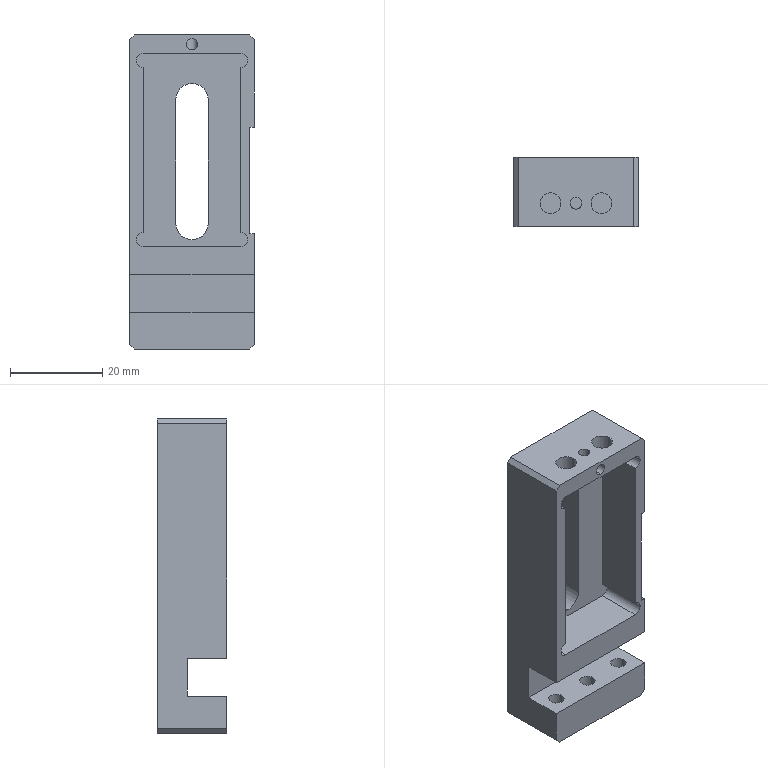Part | STEP file | 10000054277swp000-1 | 1 solid | 47 faces | box 27 x 15 x 68 mm | volume 14711 mm3 | plane 25 | cylinder 22 | commonest cylinder face diameters 3.3 x6 2.5 x5 3 x4 4.5 x4 7 x3
STEP:
#1=CARTESIAN_POINT('',(0.,7.5,-10.3));
#2=VERTEX_POINT('',#1);
#3=CARTESIAN_POINT('',(3.5,7.5,-6.8));
#4=VERTEX_POINT('',#3);
#5=CARTESIAN_POINT('',(0.,7.5,-6.8));
#6=DIRECTION('',(0.,-1.,0.));
#7=DIRECTION('',(0.,0.,-1.));
#8=AXIS2_PLACEMENT_3D('',#5,#6,#7);
#9=CIRCLE('',#8,3.5);
#10=EDGE_CURVE('',#2,#4,#9,.T.);
#11=ORIENTED_EDGE('',*,*,#10,.F.);
#12=CARTESIAN_POINT('',(0.,2.6,-10.3));
#13=VERTEX_POINT('',#12);
#14=CARTESIAN_POINT('',(0.,7.5,-10.3));
#15=DIRECTION('',(0.,-1.,0.));
#16=VECTOR('',#15,1000.);
#17=LINE('',#14,#16);
#18=EDGE_CURVE('',#2,#13,#17,.T.);
#19=ORIENTED_EDGE('',*,*,#18,.T.);
#20=CARTESIAN_POINT('',(3.5,2.6,-6.8));
#21=VERTEX_POINT('',#20);
#22=CARTESIAN_POINT('',(0.,2.6,-6.8));
#23=DIRECTION('',(0.,-1.,0.));
#24=DIRECTION('',(0.,0.,-1.));
#25=AXIS2_PLACEMENT_3D('',#22,#23,#24);
#26=CIRCLE('',#25,3.5);
#27=EDGE_CURVE('',#13,#21,#26,.T.);
#28=ORIENTED_EDGE('',*,*,#27,.T.);
#29=CARTESIAN_POINT('',(3.5,7.5,-6.8));
#30=DIRECTION('',(0.,-1.,0.));
#31=VECTOR('',#30,1000.);
#32=LINE('',#29,#31);
#33=EDGE_CURVE('',#4,#21,#32,.T.);
#34=ORIENTED_EDGE('',*,*,#33,.F.);
#35=EDGE_LOOP('',(#11,#19,#28,#34));
#36=FACE_OUTER_BOUND('',#35,.T.);
#37=CARTESIAN_POINT('',(0.,7.5,-6.8));
#38=DIRECTION('',(0.,-1.,0.));
#39=DIRECTION('',(0.,0.,-1.));
#40=AXIS2_PLACEMENT_3D('',#37,#38,#39);
#41=CYLINDRICAL_SURFACE('',#40,3.5);
#42=ADVANCED_FACE('',(#36),#41,.F.);
#43=CARTESIAN_POINT('',(0.,-3.75,33.252));
#44=VERTEX_POINT('',#43);
#45=CARTESIAN_POINT('',(-1.25,-2.5,32.002));
#46=VERTEX_POINT('',#45);
#47=CARTESIAN_POINT('',(0.,-3.75,33.252));
#48=CARTESIAN_POINT('',(-0.7322,-3.75,33.252));
#49=CARTESIAN_POINT('',(-1.25,-3.232,32.734));
#50=CARTESIAN_POINT('',(-1.25,-2.5,32.002));
#51=(BOUNDED_CURVE()B_SPLINE_CURVE(3,(#47,#48,#49,#50),.UNSPECIFIED.,.F.,.F.)B_SPLINE_CURVE_WITH_KNOTS((4,4),(0.,1.571),.UNSPECIFIED.)CURVE()GEOMETRIC_REPRESENTATION_ITEM()RATIONAL_B_SPLINE_CURVE((1.,0.8047,0.8047,1.))REPRESENTATION_ITEM(''));
#52=EDGE_CURVE('',#44,#46,#51,.T.);
#53=ORIENTED_EDGE('',*,*,#52,.F.);
#54=CARTESIAN_POINT('',(0.,-7.5,33.252));
#55=VERTEX_POINT('',#54);
#56=CARTESIAN_POINT('',(0.,-7.5,33.252));
#57=DIRECTION('',(0.,-1.,0.));
#58=VECTOR('',#57,1000.);
#59=LINE('',#56,#58);
#60=EDGE_CURVE('',#44,#55,#59,.T.);
#61=ORIENTED_EDGE('',*,*,#60,.T.);
#62=CARTESIAN_POINT('',(0.,-7.5,30.752));
#63=VERTEX_POINT('',#62);
#64=CARTESIAN_POINT('',(0.,-7.5,32.002));
#65=DIRECTION('',(0.,-1.,0.));
#66=DIRECTION('',(0.,0.,-1.));
#67=AXIS2_PLACEMENT_3D('',#64,#65,#66);
#68=CIRCLE('',#67,1.25);
#69=EDGE_CURVE('',#55,#63,#68,.T.);
#70=ORIENTED_EDGE('',*,*,#69,.T.);
#71=CARTESIAN_POINT('',(0.,-3.75,30.752));
#72=VERTEX_POINT('',#71);
#73=CARTESIAN_POINT('',(0.,-7.5,30.752));
#74=DIRECTION('',(0.,-1.,0.));
#75=VECTOR('',#74,1000.);
#76=LINE('',#73,#75);
#77=EDGE_CURVE('',#72,#63,#76,.T.);
#78=ORIENTED_EDGE('',*,*,#77,.F.);
#79=CARTESIAN_POINT('',(-1.25,-2.5,32.002));
#80=CARTESIAN_POINT('',(-1.25,-3.232,31.27));
#81=CARTESIAN_POINT('',(-0.7322,-3.75,30.752));
#82=CARTESIAN_POINT('',(0.,-3.75,30.752));
#83=(BOUNDED_CURVE()B_SPLINE_CURVE(3,(#79,#80,#81,#82),.UNSPECIFIED.,.F.,.F.)B_SPLINE_CURVE_WITH_KNOTS((4,4),(1.571,3.142),.UNSPECIFIED.)CURVE()GEOMETRIC_REPRESENTATION_ITEM()RATIONAL_B_SPLINE_CURVE((1.,0.8047,0.8047,1.))REPRESENTATION_ITEM(''));
#84=EDGE_CURVE('',#46,#72,#83,.T.);
#85=ORIENTED_EDGE('',*,*,#84,.F.);
#86=EDGE_LOOP('',(#53,#61,#70,#78,#85));
#87=FACE_OUTER_BOUND('',#86,.T.);
#88=CARTESIAN_POINT('',(0.,-7.5,32.002));
#89=DIRECTION('',(0.,-1.,0.));
#90=DIRECTION('',(0.,0.,-1.));
#91=AXIS2_PLACEMENT_3D('',#88,#89,#90);
#92=CYLINDRICAL_SURFACE('',#91,1.25);
#93=ADVANCED_FACE('',(#87),#92,.F.);
#94=CARTESIAN_POINT('',(-1.25,-2.5,30.));
#95=VERTEX_POINT('',#94);
#96=CARTESIAN_POINT('',(1.25,-2.5,30.));
#97=VERTEX_POINT('',#96);
#98=CARTESIAN_POINT('',(0.,-2.5,30.));
#99=DIRECTION('',(0.,0.,1.));
#100=DIRECTION('',(1.,0.,0.));
#101=AXIS2_PLACEMENT_3D('',#98,#99,#100);
#102=CIRCLE('',#101,1.25);
#103=EDGE_CURVE('',#95,#97,#102,.T.);
#104=ORIENTED_EDGE('',*,*,#103,.F.);
#105=CARTESIAN_POINT('',(-1.25,-2.5,34.));
#106=DIRECTION('',(0.,0.,1.));
#107=VECTOR('',#106,1000.);
#108=LINE('',#105,#107);
#109=EDGE_CURVE('',#95,#46,#108,.T.);
#110=ORIENTED_EDGE('',*,*,#109,.T.);
#111=ORIENTED_EDGE('',*,*,#84,.T.);
#112=CARTESIAN_POINT('',(1.25,-2.5,32.002));
#113=VERTEX_POINT('',#112);
#114=CARTESIAN_POINT('',(0.,-3.75,30.752));
#115=CARTESIAN_POINT('',(0.7322,-3.75,30.752));
#116=CARTESIAN_POINT('',(1.25,-3.232,31.27));
#117=CARTESIAN_POINT('',(1.25,-2.5,32.002));
#118=(BOUNDED_CURVE()B_SPLINE_CURVE(3,(#114,#115,#116,#117),.UNSPECIFIED.,.F.,.F.)B_SPLINE_CURVE_WITH_KNOTS((4,4),(3.142,4.712),.UNSPECIFIED.)CURVE()GEOMETRIC_REPRESENTATION_ITEM()RATIONAL_B_SPLINE_CURVE((1.,0.8047,0.8047,1.))REPRESENTATION_ITEM(''));
#119=EDGE_CURVE('',#72,#113,#118,.T.);
#120=ORIENTED_EDGE('',*,*,#119,.T.);
#121=CARTESIAN_POINT('',(1.25,-2.5,34.));
#122=DIRECTION('',(0.,0.,1.));
#123=VECTOR('',#122,1000.);
#124=LINE('',#121,#123);
#125=EDGE_CURVE('',#97,#113,#124,.T.);
#126=ORIENTED_EDGE('',*,*,#125,.F.);
#127=EDGE_LOOP('',(#104,#110,#111,#120,#126));
#128=FACE_OUTER_BOUND('',#127,.T.);
#129=CARTESIAN_POINT('',(0.,-2.5,34.));
#130=DIRECTION('',(0.,0.,1.));
#131=DIRECTION('',(1.,0.,0.));
#132=AXIS2_PLACEMENT_3D('',#129,#130,#131);
#133=CYLINDRICAL_SURFACE('',#132,1.25);
#134=ADVANCED_FACE('',(#128),#133,.F.);
#135=CARTESIAN_POINT('',(1.25,-2.5,32.002));
#136=CARTESIAN_POINT('',(1.25,-3.232,32.734));
#137=CARTESIAN_POINT('',(0.7322,-3.75,33.252));
#138=CARTESIAN_POINT('',(0.,-3.75,33.252));
#139=(BOUNDED_CURVE()B_SPLINE_CURVE(3,(#135,#136,#137,#138),.UNSPECIFIED.,.F.,.F.)B_SPLINE_CURVE_WITH_KNOTS((4,4),(4.712,6.283),.UNSPECIFIED.)CURVE()GEOMETRIC_REPRESENTATION_ITEM()RATIONAL_B_SPLINE_CURVE((1.,0.8047,0.8047,1.))REPRESENTATION_ITEM(''));
#140=EDGE_CURVE('',#113,#44,#139,.T.);
#141=ORIENTED_EDGE('',*,*,#140,.T.);
#142=ORIENTED_EDGE('',*,*,#52,.T.);
#143=CARTESIAN_POINT('',(-1.25,-2.5,34.));
#144=VERTEX_POINT('',#143);
#145=CARTESIAN_POINT('',(-1.25,-2.5,34.));
#146=DIRECTION('',(0.,0.,1.));
#147=VECTOR('',#146,1000.);
#148=LINE('',#145,#147);
#149=EDGE_CURVE('',#46,#144,#148,.T.);
#150=ORIENTED_EDGE('',*,*,#149,.T.);
#151=CARTESIAN_POINT('',(1.25,-2.5,34.));
#152=VERTEX_POINT('',#151);
#153=CARTESIAN_POINT('',(0.,-2.5,34.));
#154=DIRECTION('',(0.,0.,1.));
#155=DIRECTION('',(1.,0.,0.));
#156=AXIS2_PLACEMENT_3D('',#153,#154,#155);
#157=CIRCLE('',#156,1.25);
#158=EDGE_CURVE('',#144,#152,#157,.T.);
#159=ORIENTED_EDGE('',*,*,#158,.T.);
#160=CARTESIAN_POINT('',(1.25,-2.5,34.));
#161=DIRECTION('',(0.,0.,1.));
#162=VECTOR('',#161,1000.);
#163=LINE('',#160,#162);
#164=EDGE_CURVE('',#113,#152,#163,.T.);
#165=ORIENTED_EDGE('',*,*,#164,.F.);
#166=EDGE_LOOP('',(#141,#142,#150,#159,#165));
#167=FACE_OUTER_BOUND('',#166,.T.);
#168=CARTESIAN_POINT('',(0.,-2.5,34.));
#169=DIRECTION('',(0.,0.,1.));
#170=DIRECTION('',(1.,0.,0.));
#171=AXIS2_PLACEMENT_3D('',#168,#169,#170);
#172=CYLINDRICAL_SURFACE('',#171,1.25);
#173=ADVANCED_FACE('',(#167),#172,.F.);
#174=CARTESIAN_POINT('',(3.25,-2.5,30.));
#175=VERTEX_POINT('',#174);
#176=CARTESIAN_POINT('',(7.75,-2.5,30.));
#177=VERTEX_POINT('',#176);
#178=CARTESIAN_POINT('',(5.5,-2.5,30.));
#179=DIRECTION('',(0.,0.,1.));
#180=DIRECTION('',(1.,0.,0.));
#181=AXIS2_PLACEMENT_3D('',#178,#179,#180);
#182=CIRCLE('',#181,2.25);
#183=EDGE_CURVE('',#175,#177,#182,.T.);
#184=ORIENTED_EDGE('',*,*,#183,.F.);
#185=CARTESIAN_POINT('',(3.25,-2.5,34.));
#186=VERTEX_POINT('',#185);
#187=CARTESIAN_POINT('',(3.25,-2.5,34.));
#188=DIRECTION('',(0.,0.,1.));
#189=VECTOR('',#188,1000.);
#190=LINE('',#187,#189);
#191=EDGE_CURVE('',#175,#186,#190,.T.);
#192=ORIENTED_EDGE('',*,*,#191,.T.);
#193=CARTESIAN_POINT('',(7.75,-2.5,34.));
#194=VERTEX_POINT('',#193);
#195=CARTESIAN_POINT('',(5.5,-2.5,34.));
#196=DIRECTION('',(0.,0.,1.));
#197=DIRECTION('',(1.,0.,0.));
#198=AXIS2_PLACEMENT_3D('',#195,#196,#197);
#199=CIRCLE('',#198,2.25);
#200=EDGE_CURVE('',#186,#194,#199,.T.);
#201=ORIENTED_EDGE('',*,*,#200,.T.);
#202=CARTESIAN_POINT('',(7.75,-2.5,34.));
#203=DIRECTION('',(0.,0.,1.));
#204=VECTOR('',#203,1000.);
#205=LINE('',#202,#204);
#206=EDGE_CURVE('',#177,#194,#205,.T.);
#207=ORIENTED_EDGE('',*,*,#206,.F.);
#208=EDGE_LOOP('',(#184,#192,#201,#207));
#209=FACE_OUTER_BOUND('',#208,.T.);
#210=CARTESIAN_POINT('',(5.5,-2.5,34.));
#211=DIRECTION('',(0.,0.,1.));
#212=DIRECTION('',(1.,0.,0.));
#213=AXIS2_PLACEMENT_3D('',#210,#211,#212);
#214=CYLINDRICAL_SURFACE('',#213,2.25);
#215=ADVANCED_FACE('',(#209),#214,.F.);
#216=CARTESIAN_POINT('',(-7.75,-2.5,30.));
#217=VERTEX_POINT('',#216);
#218=CARTESIAN_POINT('',(-3.25,-2.5,30.));
#219=VERTEX_POINT('',#218);
#220=CARTESIAN_POINT('',(-5.5,-2.5,30.));
#221=DIRECTION('',(0.,0.,1.));
#222=DIRECTION('',(1.,0.,0.));
#223=AXIS2_PLACEMENT_3D('',#220,#221,#222);
#224=CIRCLE('',#223,2.25);
#225=EDGE_CURVE('',#217,#219,#224,.T.);
#226=ORIENTED_EDGE('',*,*,#225,.F.);
#227=CARTESIAN_POINT('',(-7.75,-2.5,34.));
#228=VERTEX_POINT('',#227);
#229=CARTESIAN_POINT('',(-7.75,-2.5,34.));
#230=DIRECTION('',(0.,0.,1.));
#231=VECTOR('',#230,1000.);
#232=LINE('',#229,#231);
#233=EDGE_CURVE('',#217,#228,#232,.T.);
#234=ORIENTED_EDGE('',*,*,#233,.T.);
#235=CARTESIAN_POINT('',(-3.25,-2.5,34.));
#236=VERTEX_POINT('',#235);
#237=CARTESIAN_POINT('',(-5.5,-2.5,34.));
#238=DIRECTION('',(0.,0.,1.));
#239=DIRECTION('',(1.,0.,0.));
#240=AXIS2_PLACEMENT_3D('',#237,#238,#239);
#241=CIRCLE('',#240,2.25);
#242=EDGE_CURVE('',#228,#236,#241,.T.);
#243=ORIENTED_EDGE('',*,*,#242,.T.);
#244=CARTESIAN_POINT('',(-3.25,-2.5,34.));
#245=DIRECTION('',(0.,0.,1.));
#246=VECTOR('',#245,1000.);
#247=LINE('',#244,#246);
#248=EDGE_CURVE('',#219,#236,#247,.T.);
#249=ORIENTED_EDGE('',*,*,#248,.F.);
#250=EDGE_LOOP('',(#226,#234,#243,#249));
#251=FACE_OUTER_BOUND('',#250,.T.);
#252=CARTESIAN_POINT('',(-5.5,-2.5,34.));
#253=DIRECTION('',(0.,0.,1.));
#254=DIRECTION('',(1.,0.,0.));
#255=AXIS2_PLACEMENT_3D('',#252,#253,#254);
#256=CYLINDRICAL_SURFACE('',#255,2.25);
#257=ADVANCED_FACE('',(#251),#256,.F.);
#258=CARTESIAN_POINT('',(-7.85,-3.5,-26.));
#259=VERTEX_POINT('',#258);
#260=CARTESIAN_POINT('',(-11.15,-3.5,-26.));
#261=VERTEX_POINT('',#260);
#262=CARTESIAN_POINT('',(-9.5,-3.5,-26.));
#263=DIRECTION('',(0.,0.,-1.));
#264=DIRECTION('',(-1.,0.,0.));
#265=AXIS2_PLACEMENT_3D('',#262,#263,#264);
#266=CIRCLE('',#265,1.65);
#267=EDGE_CURVE('',#259,#261,#266,.T.);
#268=ORIENTED_EDGE('',*,*,#267,.F.);
#269=CARTESIAN_POINT('',(-7.85,-3.5,-34.));
#270=VERTEX_POINT('',#269);
#271=CARTESIAN_POINT('',(-7.85,-3.5,-34.));
#272=DIRECTION('',(0.,0.,-1.));
#273=VECTOR('',#272,1000.);
#274=LINE('',#271,#273);
#275=EDGE_CURVE('',#259,#270,#274,.T.);
#276=ORIENTED_EDGE('',*,*,#275,.T.);
#277=CARTESIAN_POINT('',(-11.15,-3.5,-34.));
#278=VERTEX_POINT('',#277);
#279=CARTESIAN_POINT('',(-9.5,-3.5,-34.));
#280=DIRECTION('',(0.,0.,-1.));
#281=DIRECTION('',(-1.,0.,0.));
#282=AXIS2_PLACEMENT_3D('',#279,#280,#281);
#283=CIRCLE('',#282,1.65);
#284=EDGE_CURVE('',#270,#278,#283,.T.);
#285=ORIENTED_EDGE('',*,*,#284,.T.);
#286=CARTESIAN_POINT('',(-11.15,-3.5,-34.));
#287=DIRECTION('',(0.,0.,-1.));
#288=VECTOR('',#287,1000.);
#289=LINE('',#286,#288);
#290=EDGE_CURVE('',#261,#278,#289,.T.);
#291=ORIENTED_EDGE('',*,*,#290,.F.);
#292=EDGE_LOOP('',(#268,#276,#285,#291));
#293=FACE_OUTER_BOUND('',#292,.T.);
#294=CARTESIAN_POINT('',(-9.5,-3.5,-34.));
#295=DIRECTION('',(0.,0.,-1.));
#296=DIRECTION('',(-1.,0.,0.));
#297=AXIS2_PLACEMENT_3D('',#294,#295,#296);
#298=CYLINDRICAL_SURFACE('',#297,1.65);
#299=ADVANCED_FACE('',(#293),#298,.F.);
#300=CARTESIAN_POINT('',(1.65,-3.5,-26.));
#301=VERTEX_POINT('',#300);
#302=CARTESIAN_POINT('',(-1.65,-3.5,-26.));
#303=VERTEX_POINT('',#302);
#304=CARTESIAN_POINT('',(0.,-3.5,-26.));
#305=DIRECTION('',(0.,0.,-1.));
#306=DIRECTION('',(-1.,0.,0.));
#307=AXIS2_PLACEMENT_3D('',#304,#305,#306);
#308=CIRCLE('',#307,1.65);
#309=EDGE_CURVE('',#301,#303,#308,.T.);
#310=ORIENTED_EDGE('',*,*,#309,.F.);
#311=CARTESIAN_POINT('',(1.65,-3.5,-34.));
#312=VERTEX_POINT('',#311);
#313=CARTESIAN_POINT('',(1.65,-3.5,-34.));
#314=DIRECTION('',(0.,0.,-1.));
#315=VECTOR('',#314,1000.);
#316=LINE('',#313,#315);
#317=EDGE_CURVE('',#301,#312,#316,.T.);
#318=ORIENTED_EDGE('',*,*,#317,.T.);
#319=CARTESIAN_POINT('',(-1.65,-3.5,-34.));
#320=VERTEX_POINT('',#319);
#321=CARTESIAN_POINT('',(0.,-3.5,-34.));
#322=DIRECTION('',(0.,0.,-1.));
#323=DIRECTION('',(-1.,0.,0.));
#324=AXIS2_PLACEMENT_3D('',#321,#322,#323);
#325=CIRCLE('',#324,1.65);
#326=EDGE_CURVE('',#312,#320,#325,.T.);
#327=ORIENTED_EDGE('',*,*,#326,.T.);
#328=CARTESIAN_POINT('',(-1.65,-3.5,-34.));
#329=DIRECTION('',(0.,0.,-1.));
#330=VECTOR('',#329,1000.);
#331=LINE('',#328,#330);
#332=EDGE_CURVE('',#303,#320,#331,.T.);
#333=ORIENTED_EDGE('',*,*,#332,.F.);
#334=EDGE_LOOP('',(#310,#318,#327,#333));
#335=FACE_OUTER_BOUND('',#334,.T.);
#336=CARTESIAN_POINT('',(0.,-3.5,-34.));
#337=DIRECTION('',(0.,0.,-1.));
#338=DIRECTION('',(-1.,0.,0.));
#339=AXIS2_PLACEMENT_3D('',#336,#337,#338);
#340=CYLINDRICAL_SURFACE('',#339,1.65);
#341=ADVANCED_FACE('',(#335),#340,.F.);
#342=CARTESIAN_POINT('',(11.15,-3.5,-26.));
#343=VERTEX_POINT('',#342);
#344=CARTESIAN_POINT('',(7.85,-3.5,-26.));
#345=VERTEX_POINT('',#344);
#346=CARTESIAN_POINT('',(9.5,-3.5,-26.));
#347=DIRECTION('',(0.,0.,-1.));
#348=DIRECTION('',(-1.,0.,0.));
#349=AXIS2_PLACEMENT_3D('',#346,#347,#348);
#350=CIRCLE('',#349,1.65);
#351=EDGE_CURVE('',#343,#345,#350,.T.);
#352=ORIENTED_EDGE('',*,*,#351,.F.);
#353=CARTESIAN_POINT('',(11.15,-3.5,-34.));
#354=VERTEX_POINT('',#353);
#355=CARTESIAN_POINT('',(11.15,-3.5,-34.));
#356=DIRECTION('',(0.,0.,-1.));
#357=VECTOR('',#356,1000.);
#358=LINE('',#355,#357);
#359=EDGE_CURVE('',#343,#354,#358,.T.);
#360=ORIENTED_EDGE('',*,*,#359,.T.);
#361=CARTESIAN_POINT('',(7.85,-3.5,-34.));
#362=VERTEX_POINT('',#361);
#363=CARTESIAN_POINT('',(9.5,-3.5,-34.));
#364=DIRECTION('',(0.,0.,-1.));
#365=DIRECTION('',(-1.,0.,0.));
#366=AXIS2_PLACEMENT_3D('',#363,#364,#365);
#367=CIRCLE('',#366,1.65);
#368=EDGE_CURVE('',#354,#362,#367,.T.);
#369=ORIENTED_EDGE('',*,*,#368,.T.);
#370=CARTESIAN_POINT('',(7.85,-3.5,-34.));
#371=DIRECTION('',(0.,0.,-1.));
#372=VECTOR('',#371,1000.);
#373=LINE('',#370,#372);
#374=EDGE_CURVE('',#345,#362,#373,.T.);
#375=ORIENTED_EDGE('',*,*,#374,.F.);
#376=EDGE_LOOP('',(#352,#360,#369,#375));
#377=FACE_OUTER_BOUND('',#376,.T.);
#378=CARTESIAN_POINT('',(9.5,-3.5,-34.));
#379=DIRECTION('',(0.,0.,-1.));
#380=DIRECTION('',(-1.,0.,0.));
#381=AXIS2_PLACEMENT_3D('',#378,#379,#380);
#382=CYLINDRICAL_SURFACE('',#381,1.65);
#383=ADVANCED_FACE('',(#377),#382,.F.);
#384=CARTESIAN_POINT('',(13.5,7.5,33.));
#385=VERTEX_POINT('',#384);
#386=CARTESIAN_POINT('',(13.5,7.5,14.));
#387=VERTEX_POINT('',#386);
#388=CARTESIAN_POINT('',(13.5,7.5,-34.));
#389=DIRECTION('',(0.,0.,-1.));
#390=VECTOR('',#389,1000.);
#391=LINE('',#388,#390);
#392=EDGE_CURVE('',#385,#387,#391,.T.);
#393=ORIENTED_EDGE('',*,*,#392,.F.);
#394=CARTESIAN_POINT('',(13.5,-7.5,33.));
#395=VERTEX_POINT('',#394);
#396=CARTESIAN_POINT('',(13.5,7.5,33.));
#397=DIRECTION('',(0.,-1.,0.));
#398=VECTOR('',#397,1000.);
#399=LINE('',#396,#398);
#400=EDGE_CURVE('',#385,#395,#399,.T.);
#401=ORIENTED_EDGE('',*,*,#400,.T.);
#402=CARTESIAN_POINT('',(13.5,-7.5,14.));
#403=VERTEX_POINT('',#402);
#404=CARTESIAN_POINT('',(13.5,-7.5,-34.));
#405=DIRECTION('',(0.,0.,-1.));
#406=VECTOR('',#405,1000.);
#407=LINE('',#404,#406);
#408=EDGE_CURVE('',#395,#403,#407,.T.);
#409=ORIENTED_EDGE('',*,*,#408,.T.);
#410=CARTESIAN_POINT('',(13.5,-7.5,14.));
#411=DIRECTION('',(0.,1.,0.));
#412=VECTOR('',#411,1000.);
#413=LINE('',#410,#412);
#414=EDGE_CURVE('',#403,#387,#413,.T.);
#415=ORIENTED_EDGE('',*,*,#414,.T.);
#416=EDGE_LOOP('',(#393,#401,#409,#415));
#417=FACE_OUTER_BOUND('',#416,.T.);
#418=CARTESIAN_POINT('',(13.5,7.5,-34.));
#419=DIRECTION('',(-1.,0.,0.));
#420=DIRECTION('',(0.,0.,1.));
#421=AXIS2_PLACEMENT_3D('',#418,#419,#420);
#422=PLANE('',#421);
#423=ADVANCED_FACE('',(#417),#422,.F.);
#424=CARTESIAN_POINT('',(0.,-7.5,32.002));
#425=DIRECTION('',(0.,-1.,0.));
#426=DIRECTION('',(0.,0.,-1.));
#427=AXIS2_PLACEMENT_3D('',#424,#425,#426);
#428=CIRCLE('',#427,1.25);
#429=EDGE_CURVE('',#63,#55,#428,.T.);
#430=ORIENTED_EDGE('',*,*,#429,.F.);
#431=ORIENTED_EDGE('',*,*,#69,.F.);
#432=EDGE_LOOP('',(#430,#431));
#433=FACE_BOUND('',#432,.T.);
#434=CARTESIAN_POINT('',(-10.6,-7.5,-11.8));
#435=VERTEX_POINT('',#434);
#436=CARTESIAN_POINT('',(10.6,-7.5,-11.8));
#437=VERTEX_POINT('',#436);
#438=CARTESIAN_POINT('',(-10.6,-7.5,-11.8));
#439=DIRECTION('',(1.,0.,0.));
#440=VECTOR('',#439,1000.);
#441=LINE('',#438,#440);
#442=EDGE_CURVE('',#435,#437,#441,.T.);
#443=ORIENTED_EDGE('',*,*,#442,.F.);
#444=CARTESIAN_POINT('',(-10.6,-7.5,-8.8));
#445=VERTEX_POINT('',#444);
#446=CARTESIAN_POINT('',(-10.6,-7.5,-10.3));
#447=DIRECTION('',(0.,-1.,0.));
#448=DIRECTION('',(0.,0.,-1.));
#449=AXIS2_PLACEMENT_3D('',#446,#447,#448);
#450=CIRCLE('',#449,1.5);
#451=EDGE_CURVE('',#445,#435,#450,.T.);
#452=ORIENTED_EDGE('',*,*,#451,.F.);
#453=CARTESIAN_POINT('',(-10.6,-7.5,27.));
#454=VERTEX_POINT('',#453);
#455=CARTESIAN_POINT('',(-10.6,-7.5,30.));
#456=DIRECTION('',(0.,0.,-1.));
#457=VECTOR('',#456,1000.);
#458=LINE('',#455,#457);
#459=EDGE_CURVE('',#454,#445,#458,.T.);
#460=ORIENTED_EDGE('',*,*,#459,.F.);
#461=CARTESIAN_POINT('',(-10.6,-7.5,30.));
#462=VERTEX_POINT('',#461);
#463=CARTESIAN_POINT('',(-10.6,-7.5,28.5));
#464=DIRECTION('',(0.,-1.,0.));
#465=DIRECTION('',(0.,0.,-1.));
#466=AXIS2_PLACEMENT_3D('',#463,#464,#465);
#467=CIRCLE('',#466,1.5);
#468=EDGE_CURVE('',#462,#454,#467,.T.);
#469=ORIENTED_EDGE('',*,*,#468,.F.);
#470=CARTESIAN_POINT('',(10.6,-7.5,30.));
#471=VERTEX_POINT('',#470);
#472=CARTESIAN_POINT('',(-10.6,-7.5,30.));
#473=DIRECTION('',(-1.,0.,0.));
#474=VECTOR('',#473,1000.);
#475=LINE('',#472,#474);
#476=EDGE_CURVE('',#471,#462,#475,.T.);
#477=ORIENTED_EDGE('',*,*,#476,.F.);
#478=CARTESIAN_POINT('',(10.6,-7.5,27.));
#479=VERTEX_POINT('',#478);
#480=CARTESIAN_POINT('',(10.6,-7.5,28.5));
#481=DIRECTION('',(0.,-1.,0.));
#482=DIRECTION('',(0.,0.,-1.));
#483=AXIS2_PLACEMENT_3D('',#480,#481,#482);
#484=CIRCLE('',#483,1.5);
#485=EDGE_CURVE('',#479,#471,#484,.T.);
#486=ORIENTED_EDGE('',*,*,#485,.F.);
#487=CARTESIAN_POINT('',(10.6,-7.5,-8.8));
#488=VERTEX_POINT('',#487);
#489=CARTESIAN_POINT('',(10.6,-7.5,30.));
#490=DIRECTION('',(0.,0.,1.));
#491=VECTOR('',#490,1000.);
#492=LINE('',#489,#491);
#493=EDGE_CURVE('',#488,#479,#492,.T.);
#494=ORIENTED_EDGE('',*,*,#493,.F.);
#495=CARTESIAN_POINT('',(10.6,-7.5,-10.3));
#496=DIRECTION('',(0.,-1.,0.));
#497=DIRECTION('',(0.,0.,-1.));
#498=AXIS2_PLACEMENT_3D('',#495,#496,#497);
#499=CIRCLE('',#498,1.5);
#500=EDGE_CURVE('',#437,#488,#499,.T.);
#501=ORIENTED_EDGE('',*,*,#500,.F.);
#502=EDGE_LOOP('',(#443,#452,#460,#469,#477,#486,#494,#501));
#503=FACE_BOUND('',#502,.T.);
#504=CARTESIAN_POINT('',(-12.5,-7.5,34.));
#505=VERTEX_POINT('',#504);
#506=CARTESIAN_POINT('',(12.5,-7.5,34.));
#507=VERTEX_POINT('',#506);
#508=CARTESIAN_POINT('',(-13.5,-7.5,34.));
#509=DIRECTION('',(1.,0.,0.));
#510=VECTOR('',#509,1000.);
#511=LINE('',#508,#510);
#512=EDGE_CURVE('',#505,#507,#511,.T.);
#513=ORIENTED_EDGE('',*,*,#512,.F.);
#514=CARTESIAN_POINT('',(-13.5,-7.5,33.));
#515=VERTEX_POINT('',#514);
#516=CARTESIAN_POINT('',(-12.5,-7.5,34.));
#517=DIRECTION('',(-0.7071,0.,-0.7071));
#518=VECTOR('',#517,1000.);
#519=LINE('',#516,#518);
#520=EDGE_CURVE('',#505,#515,#519,.T.);
#521=ORIENTED_EDGE('',*,*,#520,.T.);
#522=CARTESIAN_POINT('',(-13.5,-7.5,-17.8));
#523=VERTEX_POINT('',#522);
#524=CARTESIAN_POINT('',(-13.5,-7.5,-34.));
#525=DIRECTION('',(0.,0.,1.));
#526=VECTOR('',#525,1000.);
#527=LINE('',#524,#526);
#528=EDGE_CURVE('',#523,#515,#527,.T.);
#529=ORIENTED_EDGE('',*,*,#528,.F.);
#530=CARTESIAN_POINT('',(13.5,-7.5,-17.8));
#531=VERTEX_POINT('',#530);
#532=CARTESIAN_POINT('',(-13.5,-7.5,-17.8));
#533=DIRECTION('',(-1.,0.,0.));
#534=VECTOR('',#533,1000.);
#535=LINE('',#532,#534);
#536=EDGE_CURVE('',#531,#523,#535,.T.);
#537=ORIENTED_EDGE('',*,*,#536,.F.);
#538=CARTESIAN_POINT('',(13.5,-7.5,-9.));
#539=VERTEX_POINT('',#538);
#540=CARTESIAN_POINT('',(13.5,-7.5,-34.));
#541=DIRECTION('',(0.,0.,-1.));
#542=VECTOR('',#541,1000.);
#543=LINE('',#540,#542);
#544=EDGE_CURVE('',#539,#531,#543,.T.);
#545=ORIENTED_EDGE('',*,*,#544,.F.);
#546=CARTESIAN_POINT('',(12.5,-7.5,-9.));
#547=VERTEX_POINT('',#546);
#548=CARTESIAN_POINT('',(13.5,-7.5,-9.));
#549=DIRECTION('',(-1.,0.,0.));
#550=VECTOR('',#549,1000.);
#551=LINE('',#548,#550);
#552=EDGE_CURVE('',#539,#547,#551,.T.);
#553=ORIENTED_EDGE('',*,*,#552,.T.);
#554=CARTESIAN_POINT('',(12.5,-7.5,14.));
#555=VERTEX_POINT('',#554);
#556=CARTESIAN_POINT('',(12.5,-7.5,14.));
#557=DIRECTION('',(0.,0.,1.));
#558=VECTOR('',#557,1000.);
#559=LINE('',#556,#558);
#560=EDGE_CURVE('',#547,#555,#559,.T.);
#561=ORIENTED_EDGE('',*,*,#560,.T.);
#562=CARTESIAN_POINT('',(13.5,-7.5,14.));
#563=DIRECTION('',(1.,0.,0.));
#564=VECTOR('',#563,1000.);
#565=LINE('',#562,#564);
#566=EDGE_CURVE('',#555,#403,#565,.T.);
#567=ORIENTED_EDGE('',*,*,#566,.T.);
#568=ORIENTED_EDGE('',*,*,#408,.F.);
#569=CARTESIAN_POINT('',(13.5,-7.5,33.));
#570=DIRECTION('',(-0.7071,0.,0.7071));
#571=VECTOR('',#570,1000.);
#572=LINE('',#569,#571);
#573=EDGE_CURVE('',#395,#507,#572,.T.);
#574=ORIENTED_EDGE('',*,*,#573,.T.);
#575=EDGE_LOOP('',(#513,#521,#529,#537,#545,#553,#561,#567,#568,#574));
#576=FACE_OUTER_BOUND('',#575,.T.);
#577=CARTESIAN_POINT('',(0.,-7.5,0.));
#578=DIRECTION('',(0.,1.,0.));
#579=DIRECTION('',(0.,0.,1.));
#580=AXIS2_PLACEMENT_3D('',#577,#578,#579);
#581=PLANE('',#580);
#582=ADVANCED_FACE('',(#433,#503,#576),#581,.F.);
#583=CARTESIAN_POINT('',(13.5,-7.5,-26.));
#584=VERTEX_POINT('',#583);
#585=CARTESIAN_POINT('',(13.5,-7.5,-33.));
#586=VERTEX_POINT('',#585);
#587=CARTESIAN_POINT('',(13.5,-7.5,-34.));
#588=DIRECTION('',(0.,0.,-1.));
#589=VECTOR('',#588,1000.);
#590=LINE('',#587,#589);
#591=EDGE_CURVE('',#584,#586,#590,.T.);
#592=ORIENTED_EDGE('',*,*,#591,.T.);
#593=CARTESIAN_POINT('',(13.5,7.5,-33.));
#594=VERTEX_POINT('',#593);
#595=CARTESIAN_POINT('',(13.5,7.5,-33.));
#596=DIRECTION('',(0.,1.,0.));
#597=VECTOR('',#596,1000.);
#598=LINE('',#595,#597);
#599=EDGE_CURVE('',#586,#594,#598,.T.);
#600=ORIENTED_EDGE('',*,*,#599,.T.);
#601=CARTESIAN_POINT('',(13.5,7.5,-9.));
#602=VERTEX_POINT('',#601);
#603=CARTESIAN_POINT('',(13.5,7.5,-34.));
#604=DIRECTION('',(0.,0.,-1.));
#605=VECTOR('',#604,1000.);
#606=LINE('',#603,#605);
#607=EDGE_CURVE('',#602,#594,#606,.T.);
#608=ORIENTED_EDGE('',*,*,#607,.F.);
#609=CARTESIAN_POINT('',(13.5,-7.5,-9.));
#610=DIRECTION('',(0.,1.,0.));
#611=VECTOR('',#610,1000.);
#612=LINE('',#609,#611);
#613=EDGE_CURVE('',#539,#602,#612,.T.);
#614=ORIENTED_EDGE('',*,*,#613,.F.);
#615=ORIENTED_EDGE('',*,*,#544,.T.);
#616=CARTESIAN_POINT('',(13.5,1.,-17.8));
#617=VERTEX_POINT('',#616);
#618=CARTESIAN_POINT('',(13.5,1.,-17.8));
#619=DIRECTION('',(0.,-1.,0.));
#620=VECTOR('',#619,1000.);
#621=LINE('',#618,#620);
#622=EDGE_CURVE('',#617,#531,#621,.T.);
#623=ORIENTED_EDGE('',*,*,#622,.F.);
#624=CARTESIAN_POINT('',(13.5,1.,-26.));
#625=VERTEX_POINT('',#624);
#626=CARTESIAN_POINT('',(13.5,1.,-17.8));
#627=DIRECTION('',(0.,0.,1.));
#628=VECTOR('',#627,1000.);
#629=LINE('',#626,#628);
#630=EDGE_CURVE('',#625,#617,#629,.T.);
#631=ORIENTED_EDGE('',*,*,#630,.F.);
#632=CARTESIAN_POINT('',(13.5,1.,-26.));
#633=DIRECTION('',(0.,-1.,0.));
#634=VECTOR('',#633,1000.);
#635=LINE('',#632,#634);
#636=EDGE_CURVE('',#625,#584,#635,.T.);
#637=ORIENTED_EDGE('',*,*,#636,.T.);
#638=EDGE_LOOP('',(#592,#600,#608,#614,#615,#623,#631,#637));
#639=FACE_OUTER_BOUND('',#638,.T.);
#640=CARTESIAN_POINT('',(13.5,7.5,-34.));
#641=DIRECTION('',(-1.,0.,0.));
#642=DIRECTION('',(0.,0.,1.));
#643=AXIS2_PLACEMENT_3D('',#640,#641,#642);
#644=PLANE('',#643);
#645=ADVANCED_FACE('',(#639),#644,.F.);
#646=CARTESIAN_POINT('',(-9.5,-3.5,-34.));
#647=DIRECTION('',(0.,0.,-1.));
#648=DIRECTION('',(-1.,0.,0.));
#649=AXIS2_PLACEMENT_3D('',#646,#647,#648);
#650=CIRCLE('',#649,1.65);
#651=EDGE_CURVE('',#278,#270,#650,.T.);
#652=ORIENTED_EDGE('',*,*,#651,.F.);
#653=ORIENTED_EDGE('',*,*,#284,.F.);
#654=EDGE_LOOP('',(#652,#653));
#655=FACE_BOUND('',#654,.T.);
#656=CARTESIAN_POINT('',(0.,-3.5,-34.));
#657=DIRECTION('',(0.,0.,-1.));
#658=DIRECTION('',(-1.,0.,0.));
#659=AXIS2_PLACEMENT_3D('',#656,#657,#658);
#660=CIRCLE('',#659,1.65);
#661=EDGE_CURVE('',#320,#312,#660,.T.);
#662=ORIENTED_EDGE('',*,*,#661,.F.);
#663=ORIENTED_EDGE('',*,*,#326,.F.);
#664=EDGE_LOOP('',(#662,#663));
#665=FACE_BOUND('',#664,.T.);
#666=CARTESIAN_POINT('',(9.5,-3.5,-34.));
#667=DIRECTION('',(0.,0.,-1.));
#668=DIRECTION('',(-1.,0.,0.));
#669=AXIS2_PLACEMENT_3D('',#666,#667,#668);
#670=CIRCLE('',#669,1.65);
#671=EDGE_CURVE('',#362,#354,#670,.T.);
#672=ORIENTED_EDGE('',*,*,#671,.F.);
#673=ORIENTED_EDGE('',*,*,#368,.F.);
#674=EDGE_LOOP('',(#672,#673));
#675=FACE_BOUND('',#674,.T.);
#676=CARTESIAN_POINT('',(12.5,-7.5,-34.));
#677=VERTEX_POINT('',#676);
#678=CARTESIAN_POINT('',(-12.5,-7.5,-34.));
#679=VERTEX_POINT('',#678);
#680=CARTESIAN_POINT('',(-13.5,-7.5,-34.));
#681=DIRECTION('',(-1.,0.,0.));
#682=VECTOR('',#681,1000.);
#683=LINE('',#680,#682);
#684=EDGE_CURVE('',#677,#679,#683,.T.);
#685=ORIENTED_EDGE('',*,*,#684,.T.);
#686=CARTESIAN_POINT('',(-12.5,7.5,-34.));
#687=VERTEX_POINT('',#686);
#688=CARTESIAN_POINT('',(-12.5,7.5,-34.));
#689=DIRECTION('',(0.,1.,0.));
#690=VECTOR('',#689,1000.);
#691=LINE('',#688,#690);
#692=EDGE_CURVE('',#679,#687,#691,.T.);
#693=ORIENTED_EDGE('',*,*,#692,.T.);
#694=CARTESIAN_POINT('',(12.5,7.5,-34.));
#695=VERTEX_POINT('',#694);
#696=CARTESIAN_POINT('',(-13.5,7.5,-34.));
#697=DIRECTION('',(-1.,0.,0.));
#698=VECTOR('',#697,1000.);
#699=LINE('',#696,#698);
#700=EDGE_CURVE('',#695,#687,#699,.T.);
#701=ORIENTED_EDGE('',*,*,#700,.F.);
#702=CARTESIAN_POINT('',(12.5,7.5,-34.));
#703=DIRECTION('',(0.,-1.,0.));
#704=VECTOR('',#703,1000.);
#705=LINE('',#702,#704);
#706=EDGE_CURVE('',#695,#677,#705,.T.);
#707=ORIENTED_EDGE('',*,*,#706,.T.);
#708=EDGE_LOOP('',(#685,#693,#701,#707));
#709=FACE_OUTER_BOUND('',#708,.T.);
#710=CARTESIAN_POINT('',(-13.5,7.5,-34.));
#711=DIRECTION('',(0.,0.,1.));
#712=DIRECTION('',(1.,0.,0.));
#713=AXIS2_PLACEMENT_3D('',#710,#711,#712);
#714=PLANE('',#713);
#715=ADVANCED_FACE('',(#655,#665,#675,#709),#714,.F.);
#716=ORIENTED_EDGE('',*,*,#528,.T.);
#717=CARTESIAN_POINT('',(-13.5,7.5,33.));
#718=VERTEX_POINT('',#717);
#719=CARTESIAN_POINT('',(-13.5,7.5,33.));
#720=DIRECTION('',(0.,1.,0.));
#721=VECTOR('',#720,1000.);
#722=LINE('',#719,#721);
#723=EDGE_CURVE('',#515,#718,#722,.T.);
#724=ORIENTED_EDGE('',*,*,#723,.T.);
#725=CARTESIAN_POINT('',(-13.5,7.5,-33.));
#726=VERTEX_POINT('',#725);
#727=CARTESIAN_POINT('',(-13.5,7.5,-34.));
#728=DIRECTION('',(0.,0.,1.));
#729=VECTOR('',#728,1000.);
#730=LINE('',#727,#729);
#731=EDGE_CURVE('',#726,#718,#730,.T.);
#732=ORIENTED_EDGE('',*,*,#731,.F.);
#733=CARTESIAN_POINT('',(-13.5,-7.5,-33.));
#734=VERTEX_POINT('',#733);
#735=CARTESIAN_POINT('',(-13.5,7.5,-33.));
#736=DIRECTION('',(0.,-1.,0.));
#737=VECTOR('',#736,1000.);
#738=LINE('',#735,#737);
#739=EDGE_CURVE('',#726,#734,#738,.T.);
#740=ORIENTED_EDGE('',*,*,#739,.T.);
#741=CARTESIAN_POINT('',(-13.5,-7.5,-26.));
#742=VERTEX_POINT('',#741);
#743=CARTESIAN_POINT('',(-13.5,-7.5,-34.));
#744=DIRECTION('',(0.,0.,1.));
#745=VECTOR('',#744,1000.);
#746=LINE('',#743,#745);
#747=EDGE_CURVE('',#734,#742,#746,.T.);
#748=ORIENTED_EDGE('',*,*,#747,.T.);
#749=CARTESIAN_POINT('',(-13.5,1.,-26.));
#750=VERTEX_POINT('',#749);
#751=CARTESIAN_POINT('',(-13.5,1.,-26.));
#752=DIRECTION('',(0.,-1.,0.));
#753=VECTOR('',#752,1000.);
#754=LINE('',#751,#753);
#755=EDGE_CURVE('',#750,#742,#754,.T.);
#756=ORIENTED_EDGE('',*,*,#755,.F.);
#757=CARTESIAN_POINT('',(-13.5,1.,-17.8));
#758=VERTEX_POINT('',#757);
#759=CARTESIAN_POINT('',(-13.5,1.,-17.8));
#760=DIRECTION('',(0.,0.,-1.));
#761=VECTOR('',#760,1000.);
#762=LINE('',#759,#761);
#763=EDGE_CURVE('',#758,#750,#762,.T.);
#764=ORIENTED_EDGE('',*,*,#763,.F.);
#765=CARTESIAN_POINT('',(-13.5,1.,-17.8));
#766=DIRECTION('',(0.,-1.,0.));
#767=VECTOR('',#766,1000.);
#768=LINE('',#765,#767);
#769=EDGE_CURVE('',#758,#523,#768,.T.);
#770=ORIENTED_EDGE('',*,*,#769,.T.);
#771=EDGE_LOOP('',(#716,#724,#732,#740,#748,#756,#764,#770));
#772=FACE_OUTER_BOUND('',#771,.T.);
#773=CARTESIAN_POINT('',(-13.5,7.5,-34.));
#774=DIRECTION('',(1.,0.,0.));
#775=DIRECTION('',(0.,0.,-1.));
#776=AXIS2_PLACEMENT_3D('',#773,#774,#775);
#777=PLANE('',#776);
#778=ADVANCED_FACE('',(#772),#777,.F.);
#779=CARTESIAN_POINT('',(0.,-2.5,34.));
#780=DIRECTION('',(0.,0.,1.));
#781=DIRECTION('',(1.,0.,0.));
#782=AXIS2_PLACEMENT_3D('',#779,#780,#781);
#783=CIRCLE('',#782,1.25);
#784=EDGE_CURVE('',#152,#144,#783,.T.);
#785=ORIENTED_EDGE('',*,*,#784,.F.);
#786=ORIENTED_EDGE('',*,*,#158,.F.);
#787=EDGE_LOOP('',(#785,#786));
#788=FACE_BOUND('',#787,.T.);
#789=CARTESIAN_POINT('',(5.5,-2.5,34.));
#790=DIRECTION('',(0.,0.,1.));
#791=DIRECTION('',(1.,0.,0.));
#792=AXIS2_PLACEMENT_3D('',#789,#790,#791);
#793=CIRCLE('',#792,2.25);
#794=EDGE_CURVE('',#194,#186,#793,.T.);
#795=ORIENTED_EDGE('',*,*,#794,.F.);
#796=ORIENTED_EDGE('',*,*,#200,.F.);
#797=EDGE_LOOP('',(#795,#796));
#798=FACE_BOUND('',#797,.T.);
#799=CARTESIAN_POINT('',(-5.5,-2.5,34.));
#800=DIRECTION('',(0.,0.,1.));
#801=DIRECTION('',(1.,0.,0.));
#802=AXIS2_PLACEMENT_3D('',#799,#800,#801);
#803=CIRCLE('',#802,2.25);
#804=EDGE_CURVE('',#236,#228,#803,.T.);
#805=ORIENTED_EDGE('',*,*,#804,.F.);
#806=ORIENTED_EDGE('',*,*,#242,.F.);
#807=EDGE_LOOP('',(#805,#806));
#808=FACE_BOUND('',#807,.T.);
#809=CARTESIAN_POINT('',(-12.5,7.5,34.));
#810=VERTEX_POINT('',#809);
#811=CARTESIAN_POINT('',(12.5,7.5,34.));
#812=VERTEX_POINT('',#811);
#813=CARTESIAN_POINT('',(-13.5,7.5,34.));
#814=DIRECTION('',(1.,0.,0.));
#815=VECTOR('',#814,1000.);
#816=LINE('',#813,#815);
#817=EDGE_CURVE('',#810,#812,#816,.T.);
#818=ORIENTED_EDGE('',*,*,#817,.F.);
#819=CARTESIAN_POINT('',(-12.5,7.5,34.));
#820=DIRECTION('',(0.,-1.,0.));
#821=VECTOR('',#820,1000.);
#822=LINE('',#819,#821);
#823=EDGE_CURVE('',#810,#505,#822,.T.);
#824=ORIENTED_EDGE('',*,*,#823,.T.);
#825=ORIENTED_EDGE('',*,*,#512,.T.);
#826=CARTESIAN_POINT('',(12.5,7.5,34.));
#827=DIRECTION('',(0.,1.,0.));
#828=VECTOR('',#827,1000.);
#829=LINE('',#826,#828);
#830=EDGE_CURVE('',#507,#812,#829,.T.);
#831=ORIENTED_EDGE('',*,*,#830,.T.);
#832=EDGE_LOOP('',(#818,#824,#825,#831));
#833=FACE_OUTER_BOUND('',#832,.T.);
#834=CARTESIAN_POINT('',(-13.5,7.5,34.));
#835=DIRECTION('',(0.,0.,-1.));
#836=DIRECTION('',(-1.,0.,0.));
#837=AXIS2_PLACEMENT_3D('',#834,#835,#836);
#838=PLANE('',#837);
#839=ADVANCED_FACE('',(#788,#798,#808,#833),#838,.F.);
#840=CARTESIAN_POINT('',(-3.5,7.5,-6.8));
#841=VERTEX_POINT('',#840);
#842=CARTESIAN_POINT('',(0.,7.5,-6.8));
#843=DIRECTION('',(0.,-1.,0.));
#844=DIRECTION('',(0.,0.,-1.));
#845=AXIS2_PLACEMENT_3D('',#842,#843,#844);
#846=CIRCLE('',#845,3.5);
#847=EDGE_CURVE('',#841,#2,#846,.T.);
#848=ORIENTED_EDGE('',*,*,#847,.T.);
#849=ORIENTED_EDGE('',*,*,#10,.T.);
#850=CARTESIAN_POINT('',(3.5,7.5,20.));
#851=VERTEX_POINT('',#850);
#852=CARTESIAN_POINT('',(3.5,7.5,-6.8));
#853=DIRECTION('',(0.,0.,1.));
#854=VECTOR('',#853,1000.);
#855=LINE('',#852,#854);
#856=EDGE_CURVE('',#4,#851,#855,.T.);
#857=ORIENTED_EDGE('',*,*,#856,.T.);
#858=CARTESIAN_POINT('',(-3.5,7.5,20.));
#859=VERTEX_POINT('',#858);
#860=CARTESIAN_POINT('',(0.,7.5,20.));
#861=DIRECTION('',(0.,-1.,0.));
#862=DIRECTION('',(0.,0.,-1.));
#863=AXIS2_PLACEMENT_3D('',#860,#861,#862);
#864=CIRCLE('',#863,3.5);
#865=EDGE_CURVE('',#851,#859,#864,.T.);
#866=ORIENTED_EDGE('',*,*,#865,.T.);
#867=CARTESIAN_POINT('',(-3.5,7.5,-6.8));
#868=DIRECTION('',(0.,0.,-1.));
#869=VECTOR('',#868,1000.);
#870=LINE('',#867,#869);
#871=EDGE_CURVE('',#859,#841,#870,.T.);
#872=ORIENTED_EDGE('',*,*,#871,.T.);
#873=EDGE_LOOP('',(#848,#849,#857,#866,#872));
#874=FACE_BOUND('',#873,.T.);
#875=ORIENTED_EDGE('',*,*,#731,.T.);
#876=CARTESIAN_POINT('',(-23.25,7.5,23.25));
#877=DIRECTION('',(0.7071,0.,0.7071));
#878=VECTOR('',#877,1000.);
#879=LINE('',#876,#878);
#880=EDGE_CURVE('',#718,#810,#879,.T.);
#881=ORIENTED_EDGE('',*,*,#880,.T.);
#882=ORIENTED_EDGE('',*,*,#817,.T.);
#883=CARTESIAN_POINT('',(23.25,7.5,23.25));
#884=DIRECTION('',(0.7071,0.,-0.7071));
#885=VECTOR('',#884,1000.);
#886=LINE('',#883,#885);
#887=EDGE_CURVE('',#812,#385,#886,.T.);
#888=ORIENTED_EDGE('',*,*,#887,.T.);
#889=ORIENTED_EDGE('',*,*,#392,.T.);
#890=CARTESIAN_POINT('',(12.5,7.5,14.));
#891=VERTEX_POINT('',#890);
#892=CARTESIAN_POINT('',(13.5,7.5,14.));
#893=DIRECTION('',(1.,0.,0.));
#894=VECTOR('',#893,1000.);
#895=LINE('',#892,#894);
#896=EDGE_CURVE('',#891,#387,#895,.T.);
#897=ORIENTED_EDGE('',*,*,#896,.F.);
#898=CARTESIAN_POINT('',(12.5,7.5,-9.));
#899=VERTEX_POINT('',#898);
#900=CARTESIAN_POINT('',(12.5,7.5,14.));
#901=DIRECTION('',(0.,0.,1.));
#902=VECTOR('',#901,1000.);
#903=LINE('',#900,#902);
#904=EDGE_CURVE('',#899,#891,#903,.T.);
#905=ORIENTED_EDGE('',*,*,#904,.F.);
#906=CARTESIAN_POINT('',(13.5,7.5,-9.));
#907=DIRECTION('',(-1.,0.,0.));
#908=VECTOR('',#907,1000.);
#909=LINE('',#906,#908);
#910=EDGE_CURVE('',#602,#899,#909,.T.);
#911=ORIENTED_EDGE('',*,*,#910,.F.);
#912=ORIENTED_EDGE('',*,*,#607,.T.);
#913=CARTESIAN_POINT('',(23.25,7.5,-23.25));
#914=DIRECTION('',(-0.7071,0.,-0.7071));
#915=VECTOR('',#914,1000.);
#916=LINE('',#913,#915);
#917=EDGE_CURVE('',#594,#695,#916,.T.);
#918=ORIENTED_EDGE('',*,*,#917,.T.);
#919=ORIENTED_EDGE('',*,*,#700,.T.);
#920=CARTESIAN_POINT('',(-23.25,7.5,-23.25));
#921=DIRECTION('',(-0.7071,0.,0.7071));
#922=VECTOR('',#921,1000.);
#923=LINE('',#920,#922);
#924=EDGE_CURVE('',#687,#726,#923,.T.);
#925=ORIENTED_EDGE('',*,*,#924,.T.);
#926=EDGE_LOOP('',(#875,#881,#882,#888,#889,#897,#905,#911,#912,#918,#919,#925));
#927=FACE_OUTER_BOUND('',#926,.T.);
#928=CARTESIAN_POINT('',(0.,7.5,0.));
#929=DIRECTION('',(0.,1.,0.));
#930=DIRECTION('',(0.,0.,1.));
#931=AXIS2_PLACEMENT_3D('',#928,#929,#930);
#932=PLANE('',#931);
#933=ADVANCED_FACE('',(#874,#927),#932,.T.);
#934=ORIENTED_EDGE('',*,*,#747,.F.);
#935=CARTESIAN_POINT('',(-13.5,-7.5,-33.));
#936=DIRECTION('',(0.7071,0.,-0.7071));
#937=VECTOR('',#936,1000.);
#938=LINE('',#935,#937);
#939=EDGE_CURVE('',#734,#679,#938,.T.);
#940=ORIENTED_EDGE('',*,*,#939,.T.);
#941=ORIENTED_EDGE('',*,*,#684,.F.);
#942=CARTESIAN_POINT('',(12.5,-7.5,-34.));
#943=DIRECTION('',(0.7071,0.,0.7071));
#944=VECTOR('',#943,1000.);
#945=LINE('',#942,#944);
#946=EDGE_CURVE('',#677,#586,#945,.T.);
#947=ORIENTED_EDGE('',*,*,#946,.T.);
#948=ORIENTED_EDGE('',*,*,#591,.F.);
#949=CARTESIAN_POINT('',(-13.5,-7.5,-26.));
#950=DIRECTION('',(1.,0.,0.));
#951=VECTOR('',#950,1000.);
#952=LINE('',#949,#951);
#953=EDGE_CURVE('',#742,#584,#952,.T.);
#954=ORIENTED_EDGE('',*,*,#953,.F.);
#955=EDGE_LOOP('',(#934,#940,#941,#947,#948,#954));
#956=FACE_OUTER_BOUND('',#955,.T.);
#957=CARTESIAN_POINT('',(0.,-7.5,0.));
#958=DIRECTION('',(0.,1.,0.));
#959=DIRECTION('',(0.,0.,1.));
#960=AXIS2_PLACEMENT_3D('',#957,#958,#959);
#961=PLANE('',#960);
#962=ADVANCED_FACE('',(#956),#961,.F.);
#963=ORIENTED_EDGE('',*,*,#536,.T.);
#964=ORIENTED_EDGE('',*,*,#769,.F.);
#965=CARTESIAN_POINT('',(-13.5,1.,-17.8));
#966=DIRECTION('',(-1.,0.,0.));
#967=VECTOR('',#966,1000.);
#968=LINE('',#965,#967);
#969=EDGE_CURVE('',#617,#758,#968,.T.);
#970=ORIENTED_EDGE('',*,*,#969,.F.);
#971=ORIENTED_EDGE('',*,*,#622,.T.);
#972=EDGE_LOOP('',(#963,#964,#970,#971));
#973=FACE_OUTER_BOUND('',#972,.T.);
#974=CARTESIAN_POINT('',(-13.5,1.,-17.8));
#975=DIRECTION('',(0.,0.,1.));
#976=DIRECTION('',(1.,0.,0.));
#977=AXIS2_PLACEMENT_3D('',#974,#975,#976);
#978=PLANE('',#977);
#979=ADVANCED_FACE('',(#973),#978,.F.);
#980=CARTESIAN_POINT('',(-9.5,-3.5,-26.));
#981=DIRECTION('',(0.,0.,-1.));
#982=DIRECTION('',(-1.,0.,0.));
#983=AXIS2_PLACEMENT_3D('',#980,#981,#982);
#984=CIRCLE('',#983,1.65);
#985=EDGE_CURVE('',#261,#259,#984,.T.);
#986=ORIENTED_EDGE('',*,*,#985,.T.);
#987=ORIENTED_EDGE('',*,*,#267,.T.);
#988=EDGE_LOOP('',(#986,#987));
#989=FACE_BOUND('',#988,.T.);
#990=CARTESIAN_POINT('',(0.,-3.5,-26.));
#991=DIRECTION('',(0.,0.,-1.));
#992=DIRECTION('',(-1.,0.,0.));
#993=AXIS2_PLACEMENT_3D('',#990,#991,#992);
#994=CIRCLE('',#993,1.65);
#995=EDGE_CURVE('',#303,#301,#994,.T.);
#996=ORIENTED_EDGE('',*,*,#995,.T.);
#997=ORIENTED_EDGE('',*,*,#309,.T.);
#998=EDGE_LOOP('',(#996,#997));
#999=FACE_BOUND('',#998,.T.);
#1000=CARTESIAN_POINT('',(9.5,-3.5,-26.));
#1001=DIRECTION('',(0.,0.,-1.));
#1002=DIRECTION('',(-1.,0.,0.));
#1003=AXIS2_PLACEMENT_3D('',#1000,#1001,#1002);
#1004=CIRCLE('',#1003,1.65);
#1005=EDGE_CURVE('',#345,#343,#1004,.T.);
#1006=ORIENTED_EDGE('',*,*,#1005,.T.);
#1007=ORIENTED_EDGE('',*,*,#351,.T.);
#1008=EDGE_LOOP('',(#1006,#1007));
#1009=FACE_BOUND('',#1008,.T.);
#1010=ORIENTED_EDGE('',*,*,#953,.T.);
#1011=ORIENTED_EDGE('',*,*,#636,.F.);
#1012=CARTESIAN_POINT('',(-13.5,1.,-26.));
#1013=DIRECTION('',(1.,0.,0.));
#1014=VECTOR('',#1013,1000.);
#1015=LINE('',#1012,#1014);
#1016=EDGE_CURVE('',#750,#625,#1015,.T.);
#1017=ORIENTED_EDGE('',*,*,#1016,.F.);
#1018=ORIENTED_EDGE('',*,*,#755,.T.);
#1019=EDGE_LOOP('',(#1010,#1011,#1017,#1018));
#1020=FACE_OUTER_BOUND('',#1019,.T.);
#1021=CARTESIAN_POINT('',(-13.5,1.,-26.));
#1022=DIRECTION('',(0.,0.,-1.));
#1023=DIRECTION('',(-1.,0.,0.));
#1024=AXIS2_PLACEMENT_3D('',#1021,#1022,#1023);
#1025=PLANE('',#1024);
#1026=ADVANCED_FACE('',(#989,#999,#1009,#1020),#1025,.F.);
#1027=ORIENTED_EDGE('',*,*,#763,.T.);
#1028=ORIENTED_EDGE('',*,*,#1016,.T.);
#1029=ORIENTED_EDGE('',*,*,#630,.T.);
#1030=ORIENTED_EDGE('',*,*,#969,.T.);
#1031=EDGE_LOOP('',(#1027,#1028,#1029,#1030));
#1032=FACE_OUTER_BOUND('',#1031,.T.);
#1033=CARTESIAN_POINT('',(0.,1.,0.));
#1034=DIRECTION('',(0.,-1.,0.));
#1035=DIRECTION('',(0.,0.,-1.));
#1036=AXIS2_PLACEMENT_3D('',#1033,#1034,#1035);
#1037=PLANE('',#1036);
#1038=ADVANCED_FACE('',(#1032),#1037,.T.);
#1039=ORIENTED_EDGE('',*,*,#359,.F.);
#1040=ORIENTED_EDGE('',*,*,#1005,.F.);
#1041=ORIENTED_EDGE('',*,*,#374,.T.);
#1042=ORIENTED_EDGE('',*,*,#671,.T.);
#1043=EDGE_LOOP('',(#1039,#1040,#1041,#1042));
#1044=FACE_OUTER_BOUND('',#1043,.T.);
#1045=CARTESIAN_POINT('',(9.5,-3.5,-34.));
#1046=DIRECTION('',(0.,0.,-1.));
#1047=DIRECTION('',(-1.,0.,0.));
#1048=AXIS2_PLACEMENT_3D('',#1045,#1046,#1047);
#1049=CYLINDRICAL_SURFACE('',#1048,1.65);
#1050=ADVANCED_FACE('',(#1044),#1049,.F.);
#1051=ORIENTED_EDGE('',*,*,#317,.F.);
#1052=ORIENTED_EDGE('',*,*,#995,.F.);
#1053=ORIENTED_EDGE('',*,*,#332,.T.);
#1054=ORIENTED_EDGE('',*,*,#661,.T.);
#1055=EDGE_LOOP('',(#1051,#1052,#1053,#1054));
#1056=FACE_OUTER_BOUND('',#1055,.T.);
#1057=CARTESIAN_POINT('',(0.,-3.5,-34.));
#1058=DIRECTION('',(0.,0.,-1.));
#1059=DIRECTION('',(-1.,0.,0.));
#1060=AXIS2_PLACEMENT_3D('',#1057,#1058,#1059);
#1061=CYLINDRICAL_SURFACE('',#1060,1.65);
#1062=ADVANCED_FACE('',(#1056),#1061,.F.);
#1063=ORIENTED_EDGE('',*,*,#275,.F.);
#1064=ORIENTED_EDGE('',*,*,#985,.F.);
#1065=ORIENTED_EDGE('',*,*,#290,.T.);
#1066=ORIENTED_EDGE('',*,*,#651,.T.);
#1067=EDGE_LOOP('',(#1063,#1064,#1065,#1066));
#1068=FACE_OUTER_BOUND('',#1067,.T.);
#1069=CARTESIAN_POINT('',(-9.5,-3.5,-34.));
#1070=DIRECTION('',(0.,0.,-1.));
#1071=DIRECTION('',(-1.,0.,0.));
#1072=AXIS2_PLACEMENT_3D('',#1069,#1070,#1071);
#1073=CYLINDRICAL_SURFACE('',#1072,1.65);
#1074=ADVANCED_FACE('',(#1068),#1073,.F.);
#1075=CARTESIAN_POINT('',(10.6,2.6,-8.8));
#1076=VERTEX_POINT('',#1075);
#1077=CARTESIAN_POINT('',(10.6,2.6,27.));
#1078=VERTEX_POINT('',#1077);
#1079=CARTESIAN_POINT('',(10.6,2.6,30.));
#1080=DIRECTION('',(0.,0.,1.));
#1081=VECTOR('',#1080,1000.);
#1082=LINE('',#1079,#1081);
#1083=EDGE_CURVE('',#1076,#1078,#1082,.T.);
#1084=ORIENTED_EDGE('',*,*,#1083,.F.);
#1085=CARTESIAN_POINT('',(10.6,6.843,-8.8));
#1086=DIRECTION('',(0.,-1.,0.));
#1087=VECTOR('',#1086,1000.);
#1088=LINE('',#1085,#1087);
#1089=EDGE_CURVE('',#1076,#488,#1088,.T.);
#1090=ORIENTED_EDGE('',*,*,#1089,.T.);
#1091=ORIENTED_EDGE('',*,*,#493,.T.);
#1092=CARTESIAN_POINT('',(10.6,6.843,27.));
#1093=DIRECTION('',(0.,1.,0.));
#1094=VECTOR('',#1093,1000.);
#1095=LINE('',#1092,#1094);
#1096=EDGE_CURVE('',#479,#1078,#1095,.T.);
#1097=ORIENTED_EDGE('',*,*,#1096,.T.);
#1098=EDGE_LOOP('',(#1084,#1090,#1091,#1097));
#1099=FACE_OUTER_BOUND('',#1098,.T.);
#1100=CARTESIAN_POINT('',(10.6,2.6,30.));
#1101=DIRECTION('',(1.,0.,0.));
#1102=DIRECTION('',(0.,0.,-1.));
#1103=AXIS2_PLACEMENT_3D('',#1100,#1101,#1102);
#1104=PLANE('',#1103);
#1105=ADVANCED_FACE('',(#1099),#1104,.F.);
#1106=ORIENTED_EDGE('',*,*,#442,.T.);
#1107=CARTESIAN_POINT('',(10.6,2.6,-11.8));
#1108=VERTEX_POINT('',#1107);
#1109=CARTESIAN_POINT('',(10.6,2.6,-11.8));
#1110=DIRECTION('',(0.,-1.,0.));
#1111=VECTOR('',#1110,1000.);
#1112=LINE('',#1109,#1111);
#1113=EDGE_CURVE('',#1108,#437,#1112,.T.);
#1114=ORIENTED_EDGE('',*,*,#1113,.F.);
#1115=CARTESIAN_POINT('',(-10.6,2.6,-11.8));
#1116=VERTEX_POINT('',#1115);
#1117=CARTESIAN_POINT('',(-10.6,2.6,-11.8));
#1118=DIRECTION('',(1.,0.,0.));
#1119=VECTOR('',#1118,1000.);
#1120=LINE('',#1117,#1119);
#1121=EDGE_CURVE('',#1116,#1108,#1120,.T.);
#1122=ORIENTED_EDGE('',*,*,#1121,.F.);
#1123=CARTESIAN_POINT('',(-10.6,2.6,-11.8));
#1124=DIRECTION('',(0.,-1.,0.));
#1125=VECTOR('',#1124,1000.);
#1126=LINE('',#1123,#1125);
#1127=EDGE_CURVE('',#1116,#435,#1126,.T.);
#1128=ORIENTED_EDGE('',*,*,#1127,.T.);
#1129=EDGE_LOOP('',(#1106,#1114,#1122,#1128));
#1130=FACE_OUTER_BOUND('',#1129,.T.);
#1131=CARTESIAN_POINT('',(-10.6,2.6,-11.8));
#1132=DIRECTION('',(0.,0.,-1.));
#1133=DIRECTION('',(-1.,0.,0.));
#1134=AXIS2_PLACEMENT_3D('',#1131,#1132,#1133);
#1135=PLANE('',#1134);
#1136=ADVANCED_FACE('',(#1130),#1135,.F.);
#1137=ORIENTED_EDGE('',*,*,#459,.T.);
#1138=CARTESIAN_POINT('',(-10.6,2.6,-8.8));
#1139=VERTEX_POINT('',#1138);
#1140=CARTESIAN_POINT('',(-10.6,6.843,-8.8));
#1141=DIRECTION('',(0.,1.,0.));
#1142=VECTOR('',#1141,1000.);
#1143=LINE('',#1140,#1142);
#1144=EDGE_CURVE('',#445,#1139,#1143,.T.);
#1145=ORIENTED_EDGE('',*,*,#1144,.T.);
#1146=CARTESIAN_POINT('',(-10.6,2.6,27.));
#1147=VERTEX_POINT('',#1146);
#1148=CARTESIAN_POINT('',(-10.6,2.6,30.));
#1149=DIRECTION('',(0.,0.,-1.));
#1150=VECTOR('',#1149,1000.);
#1151=LINE('',#1148,#1150);
#1152=EDGE_CURVE('',#1147,#1139,#1151,.T.);
#1153=ORIENTED_EDGE('',*,*,#1152,.F.);
#1154=CARTESIAN_POINT('',(-10.6,6.843,27.));
#1155=DIRECTION('',(0.,-1.,0.));
#1156=VECTOR('',#1155,1000.);
#1157=LINE('',#1154,#1156);
#1158=EDGE_CURVE('',#1147,#454,#1157,.T.);
#1159=ORIENTED_EDGE('',*,*,#1158,.T.);
#1160=EDGE_LOOP('',(#1137,#1145,#1153,#1159));
#1161=FACE_OUTER_BOUND('',#1160,.T.);
#1162=CARTESIAN_POINT('',(-10.6,2.6,30.));
#1163=DIRECTION('',(-1.,0.,0.));
#1164=DIRECTION('',(0.,0.,1.));
#1165=AXIS2_PLACEMENT_3D('',#1162,#1163,#1164);
#1166=PLANE('',#1165);
#1167=ADVANCED_FACE('',(#1161),#1166,.F.);
#1168=CARTESIAN_POINT('',(0.,-2.5,30.));
#1169=DIRECTION('',(0.,0.,1.));
#1170=DIRECTION('',(1.,0.,0.));
#1171=AXIS2_PLACEMENT_3D('',#1168,#1169,#1170);
#1172=CIRCLE('',#1171,1.25);
#1173=EDGE_CURVE('',#97,#95,#1172,.T.);
#1174=ORIENTED_EDGE('',*,*,#1173,.T.);
#1175=ORIENTED_EDGE('',*,*,#103,.T.);
#1176=EDGE_LOOP('',(#1174,#1175));
#1177=FACE_BOUND('',#1176,.T.);
#1178=CARTESIAN_POINT('',(5.5,-2.5,30.));
#1179=DIRECTION('',(0.,0.,1.));
#1180=DIRECTION('',(1.,0.,0.));
#1181=AXIS2_PLACEMENT_3D('',#1178,#1179,#1180);
#1182=CIRCLE('',#1181,2.25);
#1183=EDGE_CURVE('',#177,#175,#1182,.T.);
#1184=ORIENTED_EDGE('',*,*,#1183,.T.);
#1185=ORIENTED_EDGE('',*,*,#183,.T.);
#1186=EDGE_LOOP('',(#1184,#1185));
#1187=FACE_BOUND('',#1186,.T.);
#1188=CARTESIAN_POINT('',(-5.5,-2.5,30.));
#1189=DIRECTION('',(0.,0.,1.));
#1190=DIRECTION('',(1.,0.,0.));
#1191=AXIS2_PLACEMENT_3D('',#1188,#1189,#1190);
#1192=CIRCLE('',#1191,2.25);
#1193=EDGE_CURVE('',#219,#217,#1192,.T.);
#1194=ORIENTED_EDGE('',*,*,#1193,.T.);
#1195=ORIENTED_EDGE('',*,*,#225,.T.);
#1196=EDGE_LOOP('',(#1194,#1195));
#1197=FACE_BOUND('',#1196,.T.);
#1198=ORIENTED_EDGE('',*,*,#476,.T.);
#1199=CARTESIAN_POINT('',(-10.6,2.6,30.));
#1200=VERTEX_POINT('',#1199);
#1201=CARTESIAN_POINT('',(-10.6,2.6,30.));
#1202=DIRECTION('',(0.,-1.,0.));
#1203=VECTOR('',#1202,1000.);
#1204=LINE('',#1201,#1203);
#1205=EDGE_CURVE('',#1200,#462,#1204,.T.);
#1206=ORIENTED_EDGE('',*,*,#1205,.F.);
#1207=CARTESIAN_POINT('',(10.6,2.6,30.));
#1208=VERTEX_POINT('',#1207);
#1209=CARTESIAN_POINT('',(-10.6,2.6,30.));
#1210=DIRECTION('',(-1.,0.,0.));
#1211=VECTOR('',#1210,1000.);
#1212=LINE('',#1209,#1211);
#1213=EDGE_CURVE('',#1208,#1200,#1212,.T.);
#1214=ORIENTED_EDGE('',*,*,#1213,.F.);
#1215=CARTESIAN_POINT('',(10.6,2.6,30.));
#1216=DIRECTION('',(0.,-1.,0.));
#1217=VECTOR('',#1216,1000.);
#1218=LINE('',#1215,#1217);
#1219=EDGE_CURVE('',#1208,#471,#1218,.T.);
#1220=ORIENTED_EDGE('',*,*,#1219,.T.);
#1221=EDGE_LOOP('',(#1198,#1206,#1214,#1220));
#1222=FACE_OUTER_BOUND('',#1221,.T.);
#1223=CARTESIAN_POINT('',(-10.6,2.6,30.));
#1224=DIRECTION('',(0.,0.,1.));
#1225=DIRECTION('',(1.,0.,0.));
#1226=AXIS2_PLACEMENT_3D('',#1223,#1224,#1225);
#1227=PLANE('',#1226);
#1228=ADVANCED_FACE('',(#1177,#1187,#1197,#1222),#1227,.F.);
#1229=CARTESIAN_POINT('',(-3.5,2.6,-6.8));
#1230=VERTEX_POINT('',#1229);
#1231=CARTESIAN_POINT('',(0.,2.6,-6.8));
#1232=DIRECTION('',(0.,-1.,0.));
#1233=DIRECTION('',(0.,0.,-1.));
#1234=AXIS2_PLACEMENT_3D('',#1231,#1232,#1233);
#1235=CIRCLE('',#1234,3.5);
#1236=EDGE_CURVE('',#1230,#13,#1235,.T.);
#1237=ORIENTED_EDGE('',*,*,#1236,.F.);
#1238=CARTESIAN_POINT('',(-3.5,2.6,20.));
#1239=VERTEX_POINT('',#1238);
#1240=CARTESIAN_POINT('',(-3.5,2.6,0.));
#1241=DIRECTION('',(0.,0.,-1.));
#1242=VECTOR('',#1241,1000.);
#1243=LINE('',#1240,#1242);
#1244=EDGE_CURVE('',#1239,#1230,#1243,.T.);
#1245=ORIENTED_EDGE('',*,*,#1244,.F.);
#1246=CARTESIAN_POINT('',(3.5,2.6,20.));
#1247=VERTEX_POINT('',#1246);
#1248=CARTESIAN_POINT('',(0.,2.6,20.));
#1249=DIRECTION('',(0.,-1.,0.));
#1250=DIRECTION('',(0.,0.,-1.));
#1251=AXIS2_PLACEMENT_3D('',#1248,#1249,#1250);
#1252=CIRCLE('',#1251,3.5);
#1253=EDGE_CURVE('',#1247,#1239,#1252,.T.);
#1254=ORIENTED_EDGE('',*,*,#1253,.F.);
#1255=CARTESIAN_POINT('',(3.5,2.6,0.));
#1256=DIRECTION('',(0.,0.,1.));
#1257=VECTOR('',#1256,1000.);
#1258=LINE('',#1255,#1257);
#1259=EDGE_CURVE('',#21,#1247,#1258,.T.);
#1260=ORIENTED_EDGE('',*,*,#1259,.F.);
#1261=ORIENTED_EDGE('',*,*,#27,.F.);
#1262=EDGE_LOOP('',(#1237,#1245,#1254,#1260,#1261));
#1263=FACE_BOUND('',#1262,.T.);
#1264=ORIENTED_EDGE('',*,*,#1152,.T.);
#1265=CARTESIAN_POINT('',(-10.6,2.6,-10.3));
#1266=DIRECTION('',(0.,1.,0.));
#1267=DIRECTION('',(0.,0.,-1.));
#1268=AXIS2_PLACEMENT_3D('',#1265,#1266,#1267);
#1269=CIRCLE('',#1268,1.5);
#1270=EDGE_CURVE('',#1116,#1139,#1269,.T.);
#1271=ORIENTED_EDGE('',*,*,#1270,.F.);
#1272=ORIENTED_EDGE('',*,*,#1121,.T.);
#1273=CARTESIAN_POINT('',(10.6,2.6,-10.3));
#1274=DIRECTION('',(0.,1.,0.));
#1275=DIRECTION('',(0.,0.,-1.));
#1276=AXIS2_PLACEMENT_3D('',#1273,#1274,#1275);
#1277=CIRCLE('',#1276,1.5);
#1278=EDGE_CURVE('',#1076,#1108,#1277,.T.);
#1279=ORIENTED_EDGE('',*,*,#1278,.F.);
#1280=ORIENTED_EDGE('',*,*,#1083,.T.);
#1281=CARTESIAN_POINT('',(10.6,2.6,28.5));
#1282=DIRECTION('',(0.,1.,0.));
#1283=DIRECTION('',(0.,0.,-1.));
#1284=AXIS2_PLACEMENT_3D('',#1281,#1282,#1283);
#1285=CIRCLE('',#1284,1.5);
#1286=EDGE_CURVE('',#1208,#1078,#1285,.T.);
#1287=ORIENTED_EDGE('',*,*,#1286,.F.);
#1288=ORIENTED_EDGE('',*,*,#1213,.T.);
#1289=CARTESIAN_POINT('',(-10.6,2.6,28.5));
#1290=DIRECTION('',(0.,1.,0.));
#1291=DIRECTION('',(0.,0.,-1.));
#1292=AXIS2_PLACEMENT_3D('',#1289,#1290,#1291);
#1293=CIRCLE('',#1292,1.5);
#1294=EDGE_CURVE('',#1147,#1200,#1293,.T.);
#1295=ORIENTED_EDGE('',*,*,#1294,.F.);
#1296=EDGE_LOOP('',(#1264,#1271,#1272,#1279,#1280,#1287,#1288,#1295));
#1297=FACE_OUTER_BOUND('',#1296,.T.);
#1298=CARTESIAN_POINT('',(0.,2.6,0.));
#1299=DIRECTION('',(0.,-1.,0.));
#1300=DIRECTION('',(0.,0.,-1.));
#1301=AXIS2_PLACEMENT_3D('',#1298,#1299,#1300);
#1302=PLANE('',#1301);
#1303=ADVANCED_FACE('',(#1263,#1297),#1302,.T.);
#1304=ORIENTED_EDGE('',*,*,#1294,.T.);
#1305=ORIENTED_EDGE('',*,*,#1205,.T.);
#1306=ORIENTED_EDGE('',*,*,#468,.T.);
#1307=ORIENTED_EDGE('',*,*,#1158,.F.);
#1308=EDGE_LOOP('',(#1304,#1305,#1306,#1307));
#1309=FACE_OUTER_BOUND('',#1308,.T.);
#1310=CARTESIAN_POINT('',(-10.6,6.843,28.5));
#1311=DIRECTION('',(0.,-1.,0.));
#1312=DIRECTION('',(0.,0.,-1.));
#1313=AXIS2_PLACEMENT_3D('',#1310,#1311,#1312);
#1314=CYLINDRICAL_SURFACE('',#1313,1.5);
#1315=ADVANCED_FACE('',(#1309),#1314,.F.);
#1316=ORIENTED_EDGE('',*,*,#485,.T.);
#1317=ORIENTED_EDGE('',*,*,#1219,.F.);
#1318=ORIENTED_EDGE('',*,*,#1286,.T.);
#1319=ORIENTED_EDGE('',*,*,#1096,.F.);
#1320=EDGE_LOOP('',(#1316,#1317,#1318,#1319));
#1321=FACE_OUTER_BOUND('',#1320,.T.);
#1322=CARTESIAN_POINT('',(10.6,6.843,28.5));
#1323=DIRECTION('',(0.,-1.,0.));
#1324=DIRECTION('',(0.,0.,-1.));
#1325=AXIS2_PLACEMENT_3D('',#1322,#1323,#1324);
#1326=CYLINDRICAL_SURFACE('',#1325,1.5);
#1327=ADVANCED_FACE('',(#1321),#1326,.F.);
#1328=ORIENTED_EDGE('',*,*,#1278,.T.);
#1329=ORIENTED_EDGE('',*,*,#1113,.T.);
#1330=ORIENTED_EDGE('',*,*,#500,.T.);
#1331=ORIENTED_EDGE('',*,*,#1089,.F.);
#1332=EDGE_LOOP('',(#1328,#1329,#1330,#1331));
#1333=FACE_OUTER_BOUND('',#1332,.T.);
#1334=CARTESIAN_POINT('',(10.6,6.843,-10.3));
#1335=DIRECTION('',(0.,-1.,0.));
#1336=DIRECTION('',(0.,0.,-1.));
#1337=AXIS2_PLACEMENT_3D('',#1334,#1335,#1336);
#1338=CYLINDRICAL_SURFACE('',#1337,1.5);
#1339=ADVANCED_FACE('',(#1333),#1338,.F.);
#1340=ORIENTED_EDGE('',*,*,#1270,.T.);
#1341=ORIENTED_EDGE('',*,*,#1144,.F.);
#1342=ORIENTED_EDGE('',*,*,#451,.T.);
#1343=ORIENTED_EDGE('',*,*,#1127,.F.);
#1344=EDGE_LOOP('',(#1340,#1341,#1342,#1343));
#1345=FACE_OUTER_BOUND('',#1344,.T.);
#1346=CARTESIAN_POINT('',(-10.6,6.843,-10.3));
#1347=DIRECTION('',(0.,-1.,0.));
#1348=DIRECTION('',(0.,0.,-1.));
#1349=AXIS2_PLACEMENT_3D('',#1346,#1347,#1348);
#1350=CYLINDRICAL_SURFACE('',#1349,1.5);
#1351=ADVANCED_FACE('',(#1345),#1350,.F.);
#1352=ORIENTED_EDGE('',*,*,#233,.F.);
#1353=ORIENTED_EDGE('',*,*,#1193,.F.);
#1354=ORIENTED_EDGE('',*,*,#248,.T.);
#1355=ORIENTED_EDGE('',*,*,#804,.T.);
#1356=EDGE_LOOP('',(#1352,#1353,#1354,#1355));
#1357=FACE_OUTER_BOUND('',#1356,.T.);
#1358=CARTESIAN_POINT('',(-5.5,-2.5,34.));
#1359=DIRECTION('',(0.,0.,1.));
#1360=DIRECTION('',(1.,0.,0.));
#1361=AXIS2_PLACEMENT_3D('',#1358,#1359,#1360);
#1362=CYLINDRICAL_SURFACE('',#1361,2.25);
#1363=ADVANCED_FACE('',(#1357),#1362,.F.);
#1364=ORIENTED_EDGE('',*,*,#191,.F.);
#1365=ORIENTED_EDGE('',*,*,#1183,.F.);
#1366=ORIENTED_EDGE('',*,*,#206,.T.);
#1367=ORIENTED_EDGE('',*,*,#794,.T.);
#1368=EDGE_LOOP('',(#1364,#1365,#1366,#1367));
#1369=FACE_OUTER_BOUND('',#1368,.T.);
#1370=CARTESIAN_POINT('',(5.5,-2.5,34.));
#1371=DIRECTION('',(0.,0.,1.));
#1372=DIRECTION('',(1.,0.,0.));
#1373=AXIS2_PLACEMENT_3D('',#1370,#1371,#1372);
#1374=CYLINDRICAL_SURFACE('',#1373,2.25);
#1375=ADVANCED_FACE('',(#1369),#1374,.F.);
#1376=ORIENTED_EDGE('',*,*,#109,.F.);
#1377=ORIENTED_EDGE('',*,*,#1173,.F.);
#1378=ORIENTED_EDGE('',*,*,#125,.T.);
#1379=ORIENTED_EDGE('',*,*,#164,.T.);
#1380=ORIENTED_EDGE('',*,*,#784,.T.);
#1381=ORIENTED_EDGE('',*,*,#149,.F.);
#1382=EDGE_LOOP('',(#1376,#1377,#1378,#1379,#1380,#1381));
#1383=FACE_OUTER_BOUND('',#1382,.T.);
#1384=CARTESIAN_POINT('',(0.,-2.5,34.));
#1385=DIRECTION('',(0.,0.,1.));
#1386=DIRECTION('',(1.,0.,0.));
#1387=AXIS2_PLACEMENT_3D('',#1384,#1385,#1386);
#1388=CYLINDRICAL_SURFACE('',#1387,1.25);
#1389=ADVANCED_FACE('',(#1383),#1388,.F.);
#1390=ORIENTED_EDGE('',*,*,#896,.T.);
#1391=ORIENTED_EDGE('',*,*,#414,.F.);
#1392=ORIENTED_EDGE('',*,*,#566,.F.);
#1393=CARTESIAN_POINT('',(12.5,-7.5,14.));
#1394=DIRECTION('',(0.,1.,0.));
#1395=VECTOR('',#1394,1000.);
#1396=LINE('',#1393,#1395);
#1397=EDGE_CURVE('',#555,#891,#1396,.T.);
#1398=ORIENTED_EDGE('',*,*,#1397,.T.);
#1399=EDGE_LOOP('',(#1390,#1391,#1392,#1398));
#1400=FACE_OUTER_BOUND('',#1399,.T.);
#1401=CARTESIAN_POINT('',(13.5,-7.5,14.));
#1402=DIRECTION('',(0.,0.,1.));
#1403=DIRECTION('',(1.,0.,0.));
#1404=AXIS2_PLACEMENT_3D('',#1401,#1402,#1403);
#1405=PLANE('',#1404);
#1406=ADVANCED_FACE('',(#1400),#1405,.F.);
#1407=ORIENTED_EDGE('',*,*,#904,.T.);
#1408=ORIENTED_EDGE('',*,*,#1397,.F.);
#1409=ORIENTED_EDGE('',*,*,#560,.F.);
#1410=CARTESIAN_POINT('',(12.5,-7.5,-9.));
#1411=DIRECTION('',(0.,1.,0.));
#1412=VECTOR('',#1411,1000.);
#1413=LINE('',#1410,#1412);
#1414=EDGE_CURVE('',#547,#899,#1413,.T.);
#1415=ORIENTED_EDGE('',*,*,#1414,.T.);
#1416=EDGE_LOOP('',(#1407,#1408,#1409,#1415));
#1417=FACE_OUTER_BOUND('',#1416,.T.);
#1418=CARTESIAN_POINT('',(12.5,-7.5,14.));
#1419=DIRECTION('',(-1.,0.,0.));
#1420=DIRECTION('',(0.,0.,1.));
#1421=AXIS2_PLACEMENT_3D('',#1418,#1419,#1420);
#1422=PLANE('',#1421);
#1423=ADVANCED_FACE('',(#1417),#1422,.F.);
#1424=ORIENTED_EDGE('',*,*,#910,.T.);
#1425=ORIENTED_EDGE('',*,*,#1414,.F.);
#1426=ORIENTED_EDGE('',*,*,#552,.F.);
#1427=ORIENTED_EDGE('',*,*,#613,.T.);
#1428=EDGE_LOOP('',(#1424,#1425,#1426,#1427));
#1429=FACE_OUTER_BOUND('',#1428,.T.);
#1430=CARTESIAN_POINT('',(13.5,-7.5,-9.));
#1431=DIRECTION('',(0.,0.,-1.));
#1432=DIRECTION('',(-1.,0.,0.));
#1433=AXIS2_PLACEMENT_3D('',#1430,#1431,#1432);
#1434=PLANE('',#1433);
#1435=ADVANCED_FACE('',(#1429),#1434,.F.);
#1436=ORIENTED_EDGE('',*,*,#60,.F.);
#1437=ORIENTED_EDGE('',*,*,#140,.F.);
#1438=ORIENTED_EDGE('',*,*,#119,.F.);
#1439=ORIENTED_EDGE('',*,*,#77,.T.);
#1440=ORIENTED_EDGE('',*,*,#429,.T.);
#1441=EDGE_LOOP('',(#1436,#1437,#1438,#1439,#1440));
#1442=FACE_OUTER_BOUND('',#1441,.T.);
#1443=CARTESIAN_POINT('',(0.,-7.5,32.002));
#1444=DIRECTION('',(0.,-1.,0.));
#1445=DIRECTION('',(0.,0.,-1.));
#1446=AXIS2_PLACEMENT_3D('',#1443,#1444,#1445);
#1447=CYLINDRICAL_SURFACE('',#1446,1.25);
#1448=ADVANCED_FACE('',(#1442),#1447,.F.);
#1449=ORIENTED_EDGE('',*,*,#880,.F.);
#1450=ORIENTED_EDGE('',*,*,#723,.F.);
#1451=ORIENTED_EDGE('',*,*,#520,.F.);
#1452=ORIENTED_EDGE('',*,*,#823,.F.);
#1453=EDGE_LOOP('',(#1449,#1450,#1451,#1452));
#1454=FACE_OUTER_BOUND('',#1453,.T.);
#1455=CARTESIAN_POINT('',(-12.5,7.5,34.));
#1456=DIRECTION('',(0.7071,0.,-0.7071));
#1457=DIRECTION('',(0.,-1.,0.));
#1458=AXIS2_PLACEMENT_3D('',#1455,#1456,#1457);
#1459=PLANE('',#1458);
#1460=ADVANCED_FACE('',(#1454),#1459,.F.);
#1461=ORIENTED_EDGE('',*,*,#887,.F.);
#1462=ORIENTED_EDGE('',*,*,#830,.F.);
#1463=ORIENTED_EDGE('',*,*,#573,.F.);
#1464=ORIENTED_EDGE('',*,*,#400,.F.);
#1465=EDGE_LOOP('',(#1461,#1462,#1463,#1464));
#1466=FACE_OUTER_BOUND('',#1465,.T.);
#1467=CARTESIAN_POINT('',(13.5,7.5,33.));
#1468=DIRECTION('',(-0.7071,0.,-0.7071));
#1469=DIRECTION('',(0.,-1.,0.));
#1470=AXIS2_PLACEMENT_3D('',#1467,#1468,#1469);
#1471=PLANE('',#1470);
#1472=ADVANCED_FACE('',(#1466),#1471,.F.);
#1473=ORIENTED_EDGE('',*,*,#924,.F.);
#1474=ORIENTED_EDGE('',*,*,#692,.F.);
#1475=ORIENTED_EDGE('',*,*,#939,.F.);
#1476=ORIENTED_EDGE('',*,*,#739,.F.);
#1477=EDGE_LOOP('',(#1473,#1474,#1475,#1476));
#1478=FACE_OUTER_BOUND('',#1477,.T.);
#1479=CARTESIAN_POINT('',(-13.5,7.5,-33.));
#1480=DIRECTION('',(0.7071,0.,0.7071));
#1481=DIRECTION('',(0.,-1.,0.));
#1482=AXIS2_PLACEMENT_3D('',#1479,#1480,#1481);
#1483=PLANE('',#1482);
#1484=ADVANCED_FACE('',(#1478),#1483,.F.);
#1485=ORIENTED_EDGE('',*,*,#917,.F.);
#1486=ORIENTED_EDGE('',*,*,#599,.F.);
#1487=ORIENTED_EDGE('',*,*,#946,.F.);
#1488=ORIENTED_EDGE('',*,*,#706,.F.);
#1489=EDGE_LOOP('',(#1485,#1486,#1487,#1488));
#1490=FACE_OUTER_BOUND('',#1489,.T.);
#1491=CARTESIAN_POINT('',(12.5,7.5,-34.));
#1492=DIRECTION('',(-0.7071,0.,0.7071));
#1493=DIRECTION('',(0.,-1.,0.));
#1494=AXIS2_PLACEMENT_3D('',#1491,#1492,#1493);
#1495=PLANE('',#1494);
#1496=ADVANCED_FACE('',(#1490),#1495,.F.);
#1497=ORIENTED_EDGE('',*,*,#18,.F.);
#1498=ORIENTED_EDGE('',*,*,#847,.F.);
#1499=CARTESIAN_POINT('',(-3.5,7.5,-6.8));
#1500=DIRECTION('',(0.,-1.,0.));
#1501=VECTOR('',#1500,1000.);
#1502=LINE('',#1499,#1501);
#1503=EDGE_CURVE('',#841,#1230,#1502,.T.);
#1504=ORIENTED_EDGE('',*,*,#1503,.T.);
#1505=ORIENTED_EDGE('',*,*,#1236,.T.);
#1506=EDGE_LOOP('',(#1497,#1498,#1504,#1505));
#1507=FACE_OUTER_BOUND('',#1506,.T.);
#1508=CARTESIAN_POINT('',(0.,7.5,-6.8));
#1509=DIRECTION('',(0.,-1.,0.));
#1510=DIRECTION('',(0.,0.,-1.));
#1511=AXIS2_PLACEMENT_3D('',#1508,#1509,#1510);
#1512=CYLINDRICAL_SURFACE('',#1511,3.5);
#1513=ADVANCED_FACE('',(#1507),#1512,.F.);
#1514=ORIENTED_EDGE('',*,*,#1244,.T.);
#1515=ORIENTED_EDGE('',*,*,#1503,.F.);
#1516=ORIENTED_EDGE('',*,*,#871,.F.);
#1517=CARTESIAN_POINT('',(-3.5,7.5,20.));
#1518=DIRECTION('',(0.,-1.,0.));
#1519=VECTOR('',#1518,1000.);
#1520=LINE('',#1517,#1519);
#1521=EDGE_CURVE('',#859,#1239,#1520,.T.);
#1522=ORIENTED_EDGE('',*,*,#1521,.T.);
#1523=EDGE_LOOP('',(#1514,#1515,#1516,#1522));
#1524=FACE_OUTER_BOUND('',#1523,.T.);
#1525=CARTESIAN_POINT('',(-3.5,7.5,-6.8));
#1526=DIRECTION('',(-1.,0.,0.));
#1527=DIRECTION('',(0.,0.,1.));
#1528=AXIS2_PLACEMENT_3D('',#1525,#1526,#1527);
#1529=PLANE('',#1528);
#1530=ADVANCED_FACE('',(#1524),#1529,.F.);
#1531=ORIENTED_EDGE('',*,*,#1253,.T.);
#1532=ORIENTED_EDGE('',*,*,#1521,.F.);
#1533=ORIENTED_EDGE('',*,*,#865,.F.);
#1534=CARTESIAN_POINT('',(3.5,7.5,20.));
#1535=DIRECTION('',(0.,-1.,0.));
#1536=VECTOR('',#1535,1000.);
#1537=LINE('',#1534,#1536);
#1538=EDGE_CURVE('',#851,#1247,#1537,.T.);
#1539=ORIENTED_EDGE('',*,*,#1538,.T.);
#1540=EDGE_LOOP('',(#1531,#1532,#1533,#1539));
#1541=FACE_OUTER_BOUND('',#1540,.T.);
#1542=CARTESIAN_POINT('',(0.,7.5,20.));
#1543=DIRECTION('',(0.,-1.,0.));
#1544=DIRECTION('',(0.,0.,-1.));
#1545=AXIS2_PLACEMENT_3D('',#1542,#1543,#1544);
#1546=CYLINDRICAL_SURFACE('',#1545,3.5);
#1547=ADVANCED_FACE('',(#1541),#1546,.F.);
#1548=ORIENTED_EDGE('',*,*,#1259,.T.);
#1549=ORIENTED_EDGE('',*,*,#1538,.F.);
#1550=ORIENTED_EDGE('',*,*,#856,.F.);
#1551=ORIENTED_EDGE('',*,*,#33,.T.);
#1552=EDGE_LOOP('',(#1548,#1549,#1550,#1551));
#1553=FACE_OUTER_BOUND('',#1552,.T.);
#1554=CARTESIAN_POINT('',(3.5,7.5,-6.8));
#1555=DIRECTION('',(1.,0.,0.));
#1556=DIRECTION('',(0.,0.,-1.));
#1557=AXIS2_PLACEMENT_3D('',#1554,#1555,#1556);
#1558=PLANE('',#1557);
#1559=ADVANCED_FACE('',(#1553),#1558,.F.);
#1560=CLOSED_SHELL('',(#42,#93,#134,#173,#215,#257,#299,#341,#383,#423,#582,#645,#715,#778,#839,#933,#962,#979,#1026,#1038,#1050,#1062,#1074,#1105,#1136,#1167,#1228,#1303,#1315,#1327,#1339,#1351,#1363,#1375,#1389,#1406,#1423,#1435,#1448,#1460,#1472,#1484,#1496,#1513,#1530,#1547,#1559));
#1561=MANIFOLD_SOLID_BREP('',#1560);
#1562=CARTESIAN_POINT('',(0.,0.,0.));
#1563=DIRECTION('',(0.,0.,1.));
#1564=DIRECTION('',(1.,0.,0.));
#1565=AXIS2_PLACEMENT_3D('',#1562,#1563,#1564);
#1566=(LENGTH_UNIT()NAMED_UNIT(*)SI_UNIT(.MILLI.,.METRE.));
#1567=UNCERTAINTY_MEASURE_WITH_UNIT(LENGTH_MEASURE(0.00001),#1566,'','');
#1568=(NAMED_UNIT(*)PLANE_ANGLE_UNIT()SI_UNIT($,.RADIAN.));
#1569=(NAMED_UNIT(*)SI_UNIT($,.STERADIAN.)SOLID_ANGLE_UNIT());
#1570=(GEOMETRIC_REPRESENTATION_CONTEXT(3)GLOBAL_UNCERTAINTY_ASSIGNED_CONTEXT((#1567))GLOBAL_UNIT_ASSIGNED_CONTEXT((#1566,#1568,#1569))REPRESENTATION_CONTEXT('',''));
#1571=ADVANCED_BREP_SHAPE_REPRESENTATION('',(#1561,#1565),#1570);